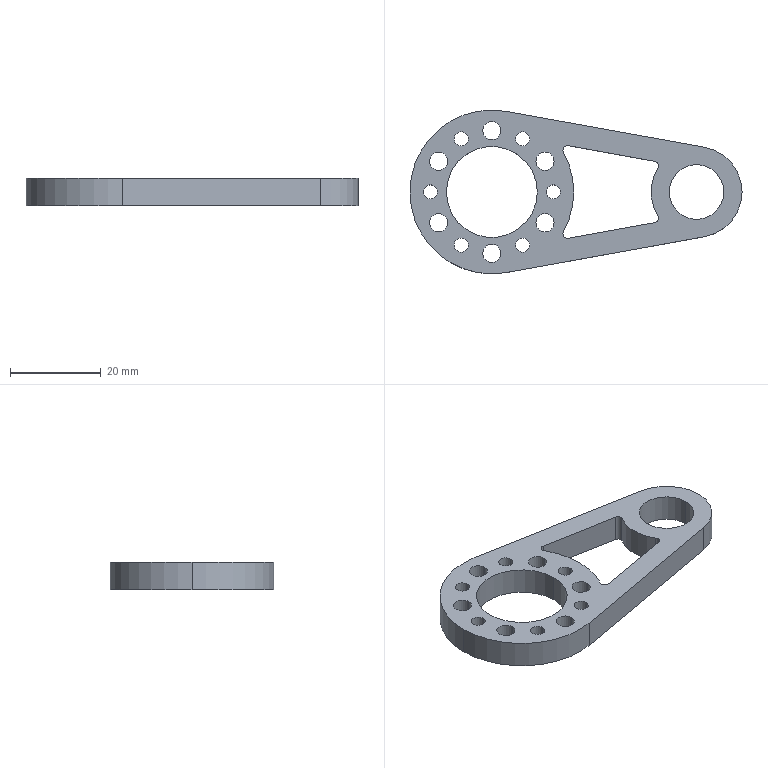Part | SolidWorks | features Extrusion 1, Fillet 1, ICE 1 | 1 solid | 46 faces | box 73 x 36 x 6 mm | volume 6499 mm3 | cylinder 40 | plane 6 | commonest cylinder face diameters 3.1 x12 4 x12 2 x6 20 x4 36 x4 12 x2
STEP:
#1=CARTESIAN_POINT('',(36.627,5.758,0.));
#2=VERTEX_POINT('',#1);
#3=CARTESIAN_POINT('',(35.805,6.742,0.));
#4=VERTEX_POINT('',#3);
#5=CARTESIAN_POINT('',(35.627,5.758,0.));
#6=DIRECTION('',(0.,0.,1.));
#7=DIRECTION('',(1.,0.,0.));
#8=AXIS2_PLACEMENT_3D('',#5,#6,#7);
#9=CIRCLE('',#8,1.);
#10=EDGE_CURVE('',#2,#4,#9,.T.);
#11=ORIENTED_EDGE('',*,*,#10,.F.);
#12=CARTESIAN_POINT('',(36.627,5.758,6.));
#13=VERTEX_POINT('',#12);
#14=CARTESIAN_POINT('',(36.627,5.758,0.));
#15=DIRECTION('',(0.,0.,1.));
#16=VECTOR('',#15,1000.);
#17=LINE('',#14,#16);
#18=EDGE_CURVE('',#2,#13,#17,.T.);
#19=ORIENTED_EDGE('',*,*,#18,.T.);
#20=CARTESIAN_POINT('',(35.805,6.742,6.));
#21=VERTEX_POINT('',#20);
#22=CARTESIAN_POINT('',(35.627,5.758,6.));
#23=DIRECTION('',(0.,0.,-1.));
#24=DIRECTION('',(1.,0.,0.));
#25=AXIS2_PLACEMENT_3D('',#22,#23,#24);
#26=CIRCLE('',#25,1.);
#27=EDGE_CURVE('',#21,#13,#26,.T.);
#28=ORIENTED_EDGE('',*,*,#27,.F.);
#29=CARTESIAN_POINT('',(35.805,6.742,6.));
#30=DIRECTION('',(0.,0.,1.));
#31=VECTOR('',#30,1000.);
#32=LINE('',#29,#31);
#33=EDGE_CURVE('',#4,#21,#32,.T.);
#34=ORIENTED_EDGE('',*,*,#33,.F.);
#35=EDGE_LOOP('',(#11,#19,#28,#34));
#36=FACE_OUTER_BOUND('',#35,.T.);
#37=CARTESIAN_POINT('',(35.627,5.758,0.));
#38=DIRECTION('',(0.,0.,1.));
#39=DIRECTION('',(1.,0.,0.));
#40=AXIS2_PLACEMENT_3D('',#37,#38,#39);
#41=CYLINDRICAL_SURFACE('',#40,1.);
#42=ADVANCED_FACE('',(#36),#41,.F.);
#43=CARTESIAN_POINT('',(36.627,-5.758,0.));
#44=VERTEX_POINT('',#43);
#45=CARTESIAN_POINT('',(36.479,-5.235,0.));
#46=VERTEX_POINT('',#45);
#47=CARTESIAN_POINT('',(35.627,-5.758,0.));
#48=DIRECTION('',(0.,0.,1.));
#49=DIRECTION('',(1.,0.,0.));
#50=AXIS2_PLACEMENT_3D('',#47,#48,#49);
#51=CIRCLE('',#50,1.);
#52=EDGE_CURVE('',#44,#46,#51,.T.);
#53=ORIENTED_EDGE('',*,*,#52,.F.);
#54=CARTESIAN_POINT('',(36.627,-5.758,6.));
#55=VERTEX_POINT('',#54);
#56=CARTESIAN_POINT('',(36.627,-5.758,0.));
#57=DIRECTION('',(0.,0.,1.));
#58=VECTOR('',#57,1000.);
#59=LINE('',#56,#58);
#60=EDGE_CURVE('',#44,#55,#59,.T.);
#61=ORIENTED_EDGE('',*,*,#60,.T.);
#62=CARTESIAN_POINT('',(36.479,-5.235,6.));
#63=VERTEX_POINT('',#62);
#64=CARTESIAN_POINT('',(35.627,-5.758,6.));
#65=DIRECTION('',(0.,0.,-1.));
#66=DIRECTION('',(1.,0.,0.));
#67=AXIS2_PLACEMENT_3D('',#64,#65,#66);
#68=CIRCLE('',#67,1.);
#69=EDGE_CURVE('',#63,#55,#68,.T.);
#70=ORIENTED_EDGE('',*,*,#69,.F.);
#71=CARTESIAN_POINT('',(36.479,-5.235,0.));
#72=DIRECTION('',(0.,0.,1.));
#73=VECTOR('',#72,1000.);
#74=LINE('',#71,#73);
#75=EDGE_CURVE('',#46,#63,#74,.T.);
#76=ORIENTED_EDGE('',*,*,#75,.F.);
#77=EDGE_LOOP('',(#53,#61,#70,#76));
#78=FACE_OUTER_BOUND('',#77,.T.);
#79=CARTESIAN_POINT('',(35.627,-5.758,0.));
#80=DIRECTION('',(0.,0.,1.));
#81=DIRECTION('',(1.,0.,0.));
#82=AXIS2_PLACEMENT_3D('',#79,#80,#81);
#83=CYLINDRICAL_SURFACE('',#82,1.);
#84=ADVANCED_FACE('',(#78),#83,.F.);
#85=CARTESIAN_POINT('',(15.754,-8.706,0.));
#86=VERTEX_POINT('',#85);
#87=CARTESIAN_POINT('',(18.,0.,0.));
#88=VERTEX_POINT('',#87);
#89=CARTESIAN_POINT('',(0.,0.,0.));
#90=DIRECTION('',(0.,0.,1.));
#91=DIRECTION('',(1.,0.,0.));
#92=AXIS2_PLACEMENT_3D('',#89,#90,#91);
#93=CIRCLE('',#92,18.);
#94=EDGE_CURVE('',#86,#88,#93,.T.);
#95=ORIENTED_EDGE('',*,*,#94,.T.);
#96=CARTESIAN_POINT('',(18.,0.,6.));
#97=VERTEX_POINT('',#96);
#98=CARTESIAN_POINT('',(18.,0.,0.));
#99=DIRECTION('',(0.,0.,1.));
#100=VECTOR('',#99,1000.);
#101=LINE('',#98,#100);
#102=EDGE_CURVE('',#88,#97,#101,.T.);
#103=ORIENTED_EDGE('',*,*,#102,.T.);
#104=CARTESIAN_POINT('',(15.754,-8.706,6.));
#105=VERTEX_POINT('',#104);
#106=CARTESIAN_POINT('',(0.,0.,6.));
#107=DIRECTION('',(0.,0.,1.));
#108=DIRECTION('',(1.,0.,0.));
#109=AXIS2_PLACEMENT_3D('',#106,#107,#108);
#110=CIRCLE('',#109,18.);
#111=EDGE_CURVE('',#105,#97,#110,.T.);
#112=ORIENTED_EDGE('',*,*,#111,.F.);
#113=CARTESIAN_POINT('',(15.754,-8.706,0.));
#114=DIRECTION('',(0.,0.,-1.));
#115=VECTOR('',#114,1000.);
#116=LINE('',#113,#115);
#117=EDGE_CURVE('',#105,#86,#116,.T.);
#118=ORIENTED_EDGE('',*,*,#117,.T.);
#119=EDGE_LOOP('',(#95,#103,#112,#118));
#120=FACE_OUTER_BOUND('',#119,.T.);
#121=CARTESIAN_POINT('',(0.,0.,0.));
#122=DIRECTION('',(0.,0.,1.));
#123=DIRECTION('',(1.,0.,0.));
#124=AXIS2_PLACEMENT_3D('',#121,#122,#123);
#125=CYLINDRICAL_SURFACE('',#124,18.);
#126=ADVANCED_FACE('',(#120),#125,.T.);
#127=CARTESIAN_POINT('',(39.,0.,6.));
#128=VERTEX_POINT('',#127);
#129=CARTESIAN_POINT('',(51.,0.,6.));
#130=VERTEX_POINT('',#129);
#131=CARTESIAN_POINT('',(45.,0.,6.));
#132=DIRECTION('',(0.,0.,1.));
#133=DIRECTION('',(1.,0.,0.));
#134=AXIS2_PLACEMENT_3D('',#131,#132,#133);
#135=CIRCLE('',#134,6.);
#136=EDGE_CURVE('',#128,#130,#135,.T.);
#137=ORIENTED_EDGE('',*,*,#136,.T.);
#138=CARTESIAN_POINT('',(51.,0.,0.));
#139=VERTEX_POINT('',#138);
#140=CARTESIAN_POINT('',(51.,0.,6.));
#141=DIRECTION('',(0.,0.,-1.));
#142=VECTOR('',#141,1000.);
#143=LINE('',#140,#142);
#144=EDGE_CURVE('',#130,#139,#143,.T.);
#145=ORIENTED_EDGE('',*,*,#144,.T.);
#146=CARTESIAN_POINT('',(39.,0.,0.));
#147=VERTEX_POINT('',#146);
#148=CARTESIAN_POINT('',(45.,0.,0.));
#149=DIRECTION('',(0.,0.,1.));
#150=DIRECTION('',(1.,0.,0.));
#151=AXIS2_PLACEMENT_3D('',#148,#149,#150);
#152=CIRCLE('',#151,6.);
#153=EDGE_CURVE('',#147,#139,#152,.T.);
#154=ORIENTED_EDGE('',*,*,#153,.F.);
#155=CARTESIAN_POINT('',(39.,0.,6.));
#156=DIRECTION('',(0.,0.,-1.));
#157=VECTOR('',#156,1000.);
#158=LINE('',#155,#157);
#159=EDGE_CURVE('',#128,#147,#158,.T.);
#160=ORIENTED_EDGE('',*,*,#159,.F.);
#161=EDGE_LOOP('',(#137,#145,#154,#160));
#162=FACE_OUTER_BOUND('',#161,.T.);
#163=CARTESIAN_POINT('',(45.,0.,6.));
#164=DIRECTION('',(0.,0.,-1.));
#165=DIRECTION('',(-1.,0.,0.));
#166=AXIS2_PLACEMENT_3D('',#163,#164,#165);
#167=CYLINDRICAL_SURFACE('',#166,6.);
#168=ADVANCED_FACE('',(#162),#167,.F.);
#169=CARTESIAN_POINT('',(-13.691,6.75,6.));
#170=VERTEX_POINT('',#169);
#171=CARTESIAN_POINT('',(-9.691,6.75,6.));
#172=VERTEX_POINT('',#171);
#173=CARTESIAN_POINT('',(-11.691,6.75,6.));
#174=DIRECTION('',(0.,0.,1.));
#175=DIRECTION('',(1.,0.,0.));
#176=AXIS2_PLACEMENT_3D('',#173,#174,#175);
#177=CIRCLE('',#176,2.);
#178=EDGE_CURVE('',#170,#172,#177,.T.);
#179=ORIENTED_EDGE('',*,*,#178,.T.);
#180=CARTESIAN_POINT('',(-9.691,6.75,0.));
#181=VERTEX_POINT('',#180);
#182=CARTESIAN_POINT('',(-9.691,6.75,6.));
#183=DIRECTION('',(0.,0.,-1.));
#184=VECTOR('',#183,1000.);
#185=LINE('',#182,#184);
#186=EDGE_CURVE('',#172,#181,#185,.T.);
#187=ORIENTED_EDGE('',*,*,#186,.T.);
#188=CARTESIAN_POINT('',(-13.691,6.75,0.));
#189=VERTEX_POINT('',#188);
#190=CARTESIAN_POINT('',(-11.691,6.75,0.));
#191=DIRECTION('',(0.,0.,1.));
#192=DIRECTION('',(1.,0.,0.));
#193=AXIS2_PLACEMENT_3D('',#190,#191,#192);
#194=CIRCLE('',#193,2.);
#195=EDGE_CURVE('',#189,#181,#194,.T.);
#196=ORIENTED_EDGE('',*,*,#195,.F.);
#197=CARTESIAN_POINT('',(-13.691,6.75,6.));
#198=DIRECTION('',(0.,0.,-1.));
#199=VECTOR('',#198,1000.);
#200=LINE('',#197,#199);
#201=EDGE_CURVE('',#170,#189,#200,.T.);
#202=ORIENTED_EDGE('',*,*,#201,.F.);
#203=EDGE_LOOP('',(#179,#187,#196,#202));
#204=FACE_OUTER_BOUND('',#203,.T.);
#205=CARTESIAN_POINT('',(-11.691,6.75,6.));
#206=DIRECTION('',(0.,0.,-1.));
#207=DIRECTION('',(-1.,0.,0.));
#208=AXIS2_PLACEMENT_3D('',#205,#206,#207);
#209=CYLINDRICAL_SURFACE('',#208,2.);
#210=ADVANCED_FACE('',(#204),#209,.F.);
#211=CARTESIAN_POINT('',(-13.691,-6.75,6.));
#212=VERTEX_POINT('',#211);
#213=CARTESIAN_POINT('',(-9.691,-6.75,6.));
#214=VERTEX_POINT('',#213);
#215=CARTESIAN_POINT('',(-11.691,-6.75,6.));
#216=DIRECTION('',(0.,0.,1.));
#217=DIRECTION('',(1.,0.,0.));
#218=AXIS2_PLACEMENT_3D('',#215,#216,#217);
#219=CIRCLE('',#218,2.);
#220=EDGE_CURVE('',#212,#214,#219,.T.);
#221=ORIENTED_EDGE('',*,*,#220,.T.);
#222=CARTESIAN_POINT('',(-9.691,-6.75,0.));
#223=VERTEX_POINT('',#222);
#224=CARTESIAN_POINT('',(-9.691,-6.75,6.));
#225=DIRECTION('',(0.,0.,-1.));
#226=VECTOR('',#225,1000.);
#227=LINE('',#224,#226);
#228=EDGE_CURVE('',#214,#223,#227,.T.);
#229=ORIENTED_EDGE('',*,*,#228,.T.);
#230=CARTESIAN_POINT('',(-13.691,-6.75,0.));
#231=VERTEX_POINT('',#230);
#232=CARTESIAN_POINT('',(-11.691,-6.75,0.));
#233=DIRECTION('',(0.,0.,1.));
#234=DIRECTION('',(1.,0.,0.));
#235=AXIS2_PLACEMENT_3D('',#232,#233,#234);
#236=CIRCLE('',#235,2.);
#237=EDGE_CURVE('',#231,#223,#236,.T.);
#238=ORIENTED_EDGE('',*,*,#237,.F.);
#239=CARTESIAN_POINT('',(-13.691,-6.75,6.));
#240=DIRECTION('',(0.,0.,-1.));
#241=VECTOR('',#240,1000.);
#242=LINE('',#239,#241);
#243=EDGE_CURVE('',#212,#231,#242,.T.);
#244=ORIENTED_EDGE('',*,*,#243,.F.);
#245=EDGE_LOOP('',(#221,#229,#238,#244));
#246=FACE_OUTER_BOUND('',#245,.T.);
#247=CARTESIAN_POINT('',(-11.691,-6.75,6.));
#248=DIRECTION('',(0.,0.,-1.));
#249=DIRECTION('',(-1.,0.,0.));
#250=AXIS2_PLACEMENT_3D('',#247,#248,#249);
#251=CYLINDRICAL_SURFACE('',#250,2.);
#252=ADVANCED_FACE('',(#246),#251,.F.);
#253=CARTESIAN_POINT('',(-2.,-13.5,6.));
#254=VERTEX_POINT('',#253);
#255=CARTESIAN_POINT('',(2.,-13.5,6.));
#256=VERTEX_POINT('',#255);
#257=CARTESIAN_POINT('',(0.,-13.5,6.));
#258=DIRECTION('',(0.,0.,1.));
#259=DIRECTION('',(1.,0.,0.));
#260=AXIS2_PLACEMENT_3D('',#257,#258,#259);
#261=CIRCLE('',#260,2.);
#262=EDGE_CURVE('',#254,#256,#261,.T.);
#263=ORIENTED_EDGE('',*,*,#262,.T.);
#264=CARTESIAN_POINT('',(2.,-13.5,0.));
#265=VERTEX_POINT('',#264);
#266=CARTESIAN_POINT('',(2.,-13.5,6.));
#267=DIRECTION('',(0.,0.,-1.));
#268=VECTOR('',#267,1000.);
#269=LINE('',#266,#268);
#270=EDGE_CURVE('',#256,#265,#269,.T.);
#271=ORIENTED_EDGE('',*,*,#270,.T.);
#272=CARTESIAN_POINT('',(-2.,-13.5,0.));
#273=VERTEX_POINT('',#272);
#274=CARTESIAN_POINT('',(0.,-13.5,0.));
#275=DIRECTION('',(0.,0.,1.));
#276=DIRECTION('',(1.,0.,0.));
#277=AXIS2_PLACEMENT_3D('',#274,#275,#276);
#278=CIRCLE('',#277,2.);
#279=EDGE_CURVE('',#273,#265,#278,.T.);
#280=ORIENTED_EDGE('',*,*,#279,.F.);
#281=CARTESIAN_POINT('',(-2.,-13.5,6.));
#282=DIRECTION('',(0.,0.,-1.));
#283=VECTOR('',#282,1000.);
#284=LINE('',#281,#283);
#285=EDGE_CURVE('',#254,#273,#284,.T.);
#286=ORIENTED_EDGE('',*,*,#285,.F.);
#287=EDGE_LOOP('',(#263,#271,#280,#286));
#288=FACE_OUTER_BOUND('',#287,.T.);
#289=CARTESIAN_POINT('',(0.,-13.5,6.));
#290=DIRECTION('',(0.,0.,-1.));
#291=DIRECTION('',(-1.,0.,0.));
#292=AXIS2_PLACEMENT_3D('',#289,#290,#291);
#293=CYLINDRICAL_SURFACE('',#292,2.);
#294=ADVANCED_FACE('',(#288),#293,.F.);
#295=CARTESIAN_POINT('',(9.691,-6.75,6.));
#296=VERTEX_POINT('',#295);
#297=CARTESIAN_POINT('',(13.691,-6.75,6.));
#298=VERTEX_POINT('',#297);
#299=CARTESIAN_POINT('',(11.691,-6.75,6.));
#300=DIRECTION('',(0.,0.,1.));
#301=DIRECTION('',(1.,0.,0.));
#302=AXIS2_PLACEMENT_3D('',#299,#300,#301);
#303=CIRCLE('',#302,2.);
#304=EDGE_CURVE('',#296,#298,#303,.T.);
#305=ORIENTED_EDGE('',*,*,#304,.T.);
#306=CARTESIAN_POINT('',(13.691,-6.75,0.));
#307=VERTEX_POINT('',#306);
#308=CARTESIAN_POINT('',(13.691,-6.75,6.));
#309=DIRECTION('',(0.,0.,-1.));
#310=VECTOR('',#309,1000.);
#311=LINE('',#308,#310);
#312=EDGE_CURVE('',#298,#307,#311,.T.);
#313=ORIENTED_EDGE('',*,*,#312,.T.);
#314=CARTESIAN_POINT('',(9.691,-6.75,0.));
#315=VERTEX_POINT('',#314);
#316=CARTESIAN_POINT('',(11.691,-6.75,0.));
#317=DIRECTION('',(0.,0.,1.));
#318=DIRECTION('',(1.,0.,0.));
#319=AXIS2_PLACEMENT_3D('',#316,#317,#318);
#320=CIRCLE('',#319,2.);
#321=EDGE_CURVE('',#315,#307,#320,.T.);
#322=ORIENTED_EDGE('',*,*,#321,.F.);
#323=CARTESIAN_POINT('',(9.691,-6.75,6.));
#324=DIRECTION('',(0.,0.,-1.));
#325=VECTOR('',#324,1000.);
#326=LINE('',#323,#325);
#327=EDGE_CURVE('',#296,#315,#326,.T.);
#328=ORIENTED_EDGE('',*,*,#327,.F.);
#329=EDGE_LOOP('',(#305,#313,#322,#328));
#330=FACE_OUTER_BOUND('',#329,.T.);
#331=CARTESIAN_POINT('',(11.691,-6.75,6.));
#332=DIRECTION('',(0.,0.,-1.));
#333=DIRECTION('',(-1.,0.,0.));
#334=AXIS2_PLACEMENT_3D('',#331,#332,#333);
#335=CYLINDRICAL_SURFACE('',#334,2.);
#336=ADVANCED_FACE('',(#330),#335,.F.);
#337=CARTESIAN_POINT('',(9.691,6.75,6.));
#338=VERTEX_POINT('',#337);
#339=CARTESIAN_POINT('',(13.691,6.75,6.));
#340=VERTEX_POINT('',#339);
#341=CARTESIAN_POINT('',(11.691,6.75,6.));
#342=DIRECTION('',(0.,0.,1.));
#343=DIRECTION('',(1.,0.,0.));
#344=AXIS2_PLACEMENT_3D('',#341,#342,#343);
#345=CIRCLE('',#344,2.);
#346=EDGE_CURVE('',#338,#340,#345,.T.);
#347=ORIENTED_EDGE('',*,*,#346,.T.);
#348=CARTESIAN_POINT('',(13.691,6.75,0.));
#349=VERTEX_POINT('',#348);
#350=CARTESIAN_POINT('',(13.691,6.75,6.));
#351=DIRECTION('',(0.,0.,-1.));
#352=VECTOR('',#351,1000.);
#353=LINE('',#350,#352);
#354=EDGE_CURVE('',#340,#349,#353,.T.);
#355=ORIENTED_EDGE('',*,*,#354,.T.);
#356=CARTESIAN_POINT('',(9.691,6.75,0.));
#357=VERTEX_POINT('',#356);
#358=CARTESIAN_POINT('',(11.691,6.75,0.));
#359=DIRECTION('',(0.,0.,1.));
#360=DIRECTION('',(1.,0.,0.));
#361=AXIS2_PLACEMENT_3D('',#358,#359,#360);
#362=CIRCLE('',#361,2.);
#363=EDGE_CURVE('',#357,#349,#362,.T.);
#364=ORIENTED_EDGE('',*,*,#363,.F.);
#365=CARTESIAN_POINT('',(9.691,6.75,6.));
#366=DIRECTION('',(0.,0.,-1.));
#367=VECTOR('',#366,1000.);
#368=LINE('',#365,#367);
#369=EDGE_CURVE('',#338,#357,#368,.T.);
#370=ORIENTED_EDGE('',*,*,#369,.F.);
#371=EDGE_LOOP('',(#347,#355,#364,#370));
#372=FACE_OUTER_BOUND('',#371,.T.);
#373=CARTESIAN_POINT('',(11.691,6.75,6.));
#374=DIRECTION('',(0.,0.,-1.));
#375=DIRECTION('',(-1.,0.,0.));
#376=AXIS2_PLACEMENT_3D('',#373,#374,#375);
#377=CYLINDRICAL_SURFACE('',#376,2.);
#378=ADVANCED_FACE('',(#372),#377,.F.);
#379=CARTESIAN_POINT('',(-2.,13.5,6.));
#380=VERTEX_POINT('',#379);
#381=CARTESIAN_POINT('',(2.,13.5,6.));
#382=VERTEX_POINT('',#381);
#383=CARTESIAN_POINT('',(0.,13.5,6.));
#384=DIRECTION('',(0.,0.,1.));
#385=DIRECTION('',(1.,0.,0.));
#386=AXIS2_PLACEMENT_3D('',#383,#384,#385);
#387=CIRCLE('',#386,2.);
#388=EDGE_CURVE('',#380,#382,#387,.T.);
#389=ORIENTED_EDGE('',*,*,#388,.T.);
#390=CARTESIAN_POINT('',(2.,13.5,0.));
#391=VERTEX_POINT('',#390);
#392=CARTESIAN_POINT('',(2.,13.5,6.));
#393=DIRECTION('',(0.,0.,-1.));
#394=VECTOR('',#393,1000.);
#395=LINE('',#392,#394);
#396=EDGE_CURVE('',#382,#391,#395,.T.);
#397=ORIENTED_EDGE('',*,*,#396,.T.);
#398=CARTESIAN_POINT('',(-2.,13.5,0.));
#399=VERTEX_POINT('',#398);
#400=CARTESIAN_POINT('',(0.,13.5,0.));
#401=DIRECTION('',(0.,0.,1.));
#402=DIRECTION('',(1.,0.,0.));
#403=AXIS2_PLACEMENT_3D('',#400,#401,#402);
#404=CIRCLE('',#403,2.);
#405=EDGE_CURVE('',#399,#391,#404,.T.);
#406=ORIENTED_EDGE('',*,*,#405,.F.);
#407=CARTESIAN_POINT('',(-2.,13.5,6.));
#408=DIRECTION('',(0.,0.,-1.));
#409=VECTOR('',#408,1000.);
#410=LINE('',#407,#409);
#411=EDGE_CURVE('',#380,#399,#410,.T.);
#412=ORIENTED_EDGE('',*,*,#411,.F.);
#413=EDGE_LOOP('',(#389,#397,#406,#412));
#414=FACE_OUTER_BOUND('',#413,.T.);
#415=CARTESIAN_POINT('',(0.,13.5,6.));
#416=DIRECTION('',(0.,0.,-1.));
#417=DIRECTION('',(-1.,0.,0.));
#418=AXIS2_PLACEMENT_3D('',#415,#416,#417);
#419=CYLINDRICAL_SURFACE('',#418,2.);
#420=ADVANCED_FACE('',(#414),#419,.F.);
#421=CARTESIAN_POINT('',(-10.,0.,6.));
#422=VERTEX_POINT('',#421);
#423=CARTESIAN_POINT('',(10.,0.,6.));
#424=VERTEX_POINT('',#423);
#425=CARTESIAN_POINT('',(0.,0.,6.));
#426=DIRECTION('',(0.,0.,1.));
#427=DIRECTION('',(1.,0.,0.));
#428=AXIS2_PLACEMENT_3D('',#425,#426,#427);
#429=CIRCLE('',#428,10.);
#430=EDGE_CURVE('',#422,#424,#429,.T.);
#431=ORIENTED_EDGE('',*,*,#430,.T.);
#432=CARTESIAN_POINT('',(10.,0.,0.));
#433=VERTEX_POINT('',#432);
#434=CARTESIAN_POINT('',(10.,0.,6.));
#435=DIRECTION('',(0.,0.,-1.));
#436=VECTOR('',#435,1000.);
#437=LINE('',#434,#436);
#438=EDGE_CURVE('',#424,#433,#437,.T.);
#439=ORIENTED_EDGE('',*,*,#438,.T.);
#440=CARTESIAN_POINT('',(-10.,0.,0.));
#441=VERTEX_POINT('',#440);
#442=CARTESIAN_POINT('',(0.,0.,0.));
#443=DIRECTION('',(0.,0.,1.));
#444=DIRECTION('',(1.,0.,0.));
#445=AXIS2_PLACEMENT_3D('',#442,#443,#444);
#446=CIRCLE('',#445,10.);
#447=EDGE_CURVE('',#441,#433,#446,.T.);
#448=ORIENTED_EDGE('',*,*,#447,.F.);
#449=CARTESIAN_POINT('',(-10.,0.,6.));
#450=DIRECTION('',(0.,0.,-1.));
#451=VECTOR('',#450,1000.);
#452=LINE('',#449,#451);
#453=EDGE_CURVE('',#422,#441,#452,.T.);
#454=ORIENTED_EDGE('',*,*,#453,.F.);
#455=EDGE_LOOP('',(#431,#439,#448,#454));
#456=FACE_OUTER_BOUND('',#455,.T.);
#457=CARTESIAN_POINT('',(0.,0.,6.));
#458=DIRECTION('',(0.,0.,-1.));
#459=DIRECTION('',(-1.,0.,0.));
#460=AXIS2_PLACEMENT_3D('',#457,#458,#459);
#461=CYLINDRICAL_SURFACE('',#460,10.);
#462=ADVANCED_FACE('',(#456),#461,.F.);
#463=CARTESIAN_POINT('',(11.95,0.,6.));
#464=VERTEX_POINT('',#463);
#465=CARTESIAN_POINT('',(15.05,0.,6.));
#466=VERTEX_POINT('',#465);
#467=CARTESIAN_POINT('',(13.5,0.,6.));
#468=DIRECTION('',(0.,0.,1.));
#469=DIRECTION('',(1.,0.,0.));
#470=AXIS2_PLACEMENT_3D('',#467,#468,#469);
#471=CIRCLE('',#470,1.55);
#472=EDGE_CURVE('',#464,#466,#471,.T.);
#473=ORIENTED_EDGE('',*,*,#472,.T.);
#474=CARTESIAN_POINT('',(15.05,0.,0.));
#475=VERTEX_POINT('',#474);
#476=CARTESIAN_POINT('',(15.05,0.,6.));
#477=DIRECTION('',(0.,0.,-1.));
#478=VECTOR('',#477,1000.);
#479=LINE('',#476,#478);
#480=EDGE_CURVE('',#466,#475,#479,.T.);
#481=ORIENTED_EDGE('',*,*,#480,.T.);
#482=CARTESIAN_POINT('',(11.95,0.,0.));
#483=VERTEX_POINT('',#482);
#484=CARTESIAN_POINT('',(13.5,0.,0.));
#485=DIRECTION('',(0.,0.,1.));
#486=DIRECTION('',(1.,0.,0.));
#487=AXIS2_PLACEMENT_3D('',#484,#485,#486);
#488=CIRCLE('',#487,1.55);
#489=EDGE_CURVE('',#483,#475,#488,.T.);
#490=ORIENTED_EDGE('',*,*,#489,.F.);
#491=CARTESIAN_POINT('',(11.95,0.,6.));
#492=DIRECTION('',(0.,0.,-1.));
#493=VECTOR('',#492,1000.);
#494=LINE('',#491,#493);
#495=EDGE_CURVE('',#464,#483,#494,.T.);
#496=ORIENTED_EDGE('',*,*,#495,.F.);
#497=EDGE_LOOP('',(#473,#481,#490,#496));
#498=FACE_OUTER_BOUND('',#497,.T.);
#499=CARTESIAN_POINT('',(13.5,0.,6.));
#500=DIRECTION('',(0.,0.,-1.));
#501=DIRECTION('',(-1.,0.,0.));
#502=AXIS2_PLACEMENT_3D('',#499,#500,#501);
#503=CYLINDRICAL_SURFACE('',#502,1.55);
#504=ADVANCED_FACE('',(#498),#503,.F.);
#505=CARTESIAN_POINT('',(5.2,-11.691,6.));
#506=VERTEX_POINT('',#505);
#507=CARTESIAN_POINT('',(8.3,-11.691,6.));
#508=VERTEX_POINT('',#507);
#509=CARTESIAN_POINT('',(6.75,-11.691,6.));
#510=DIRECTION('',(0.,0.,1.));
#511=DIRECTION('',(1.,0.,0.));
#512=AXIS2_PLACEMENT_3D('',#509,#510,#511);
#513=CIRCLE('',#512,1.55);
#514=EDGE_CURVE('',#506,#508,#513,.T.);
#515=ORIENTED_EDGE('',*,*,#514,.T.);
#516=CARTESIAN_POINT('',(8.3,-11.691,0.));
#517=VERTEX_POINT('',#516);
#518=CARTESIAN_POINT('',(8.3,-11.691,6.));
#519=DIRECTION('',(0.,0.,-1.));
#520=VECTOR('',#519,1000.);
#521=LINE('',#518,#520);
#522=EDGE_CURVE('',#508,#517,#521,.T.);
#523=ORIENTED_EDGE('',*,*,#522,.T.);
#524=CARTESIAN_POINT('',(5.2,-11.691,0.));
#525=VERTEX_POINT('',#524);
#526=CARTESIAN_POINT('',(6.75,-11.691,0.));
#527=DIRECTION('',(0.,0.,1.));
#528=DIRECTION('',(1.,0.,0.));
#529=AXIS2_PLACEMENT_3D('',#526,#527,#528);
#530=CIRCLE('',#529,1.55);
#531=EDGE_CURVE('',#525,#517,#530,.T.);
#532=ORIENTED_EDGE('',*,*,#531,.F.);
#533=CARTESIAN_POINT('',(5.2,-11.691,6.));
#534=DIRECTION('',(0.,0.,-1.));
#535=VECTOR('',#534,1000.);
#536=LINE('',#533,#535);
#537=EDGE_CURVE('',#506,#525,#536,.T.);
#538=ORIENTED_EDGE('',*,*,#537,.F.);
#539=EDGE_LOOP('',(#515,#523,#532,#538));
#540=FACE_OUTER_BOUND('',#539,.T.);
#541=CARTESIAN_POINT('',(6.75,-11.691,6.));
#542=DIRECTION('',(0.,0.,-1.));
#543=DIRECTION('',(-1.,0.,0.));
#544=AXIS2_PLACEMENT_3D('',#541,#542,#543);
#545=CYLINDRICAL_SURFACE('',#544,1.55);
#546=ADVANCED_FACE('',(#540),#545,.F.);
#547=CARTESIAN_POINT('',(-8.3,-11.691,6.));
#548=VERTEX_POINT('',#547);
#549=CARTESIAN_POINT('',(-5.2,-11.691,6.));
#550=VERTEX_POINT('',#549);
#551=CARTESIAN_POINT('',(-6.75,-11.691,6.));
#552=DIRECTION('',(0.,0.,1.));
#553=DIRECTION('',(1.,0.,0.));
#554=AXIS2_PLACEMENT_3D('',#551,#552,#553);
#555=CIRCLE('',#554,1.55);
#556=EDGE_CURVE('',#548,#550,#555,.T.);
#557=ORIENTED_EDGE('',*,*,#556,.T.);
#558=CARTESIAN_POINT('',(-5.2,-11.691,0.));
#559=VERTEX_POINT('',#558);
#560=CARTESIAN_POINT('',(-5.2,-11.691,6.));
#561=DIRECTION('',(0.,0.,-1.));
#562=VECTOR('',#561,1000.);
#563=LINE('',#560,#562);
#564=EDGE_CURVE('',#550,#559,#563,.T.);
#565=ORIENTED_EDGE('',*,*,#564,.T.);
#566=CARTESIAN_POINT('',(-8.3,-11.691,0.));
#567=VERTEX_POINT('',#566);
#568=CARTESIAN_POINT('',(-6.75,-11.691,0.));
#569=DIRECTION('',(0.,0.,1.));
#570=DIRECTION('',(1.,0.,0.));
#571=AXIS2_PLACEMENT_3D('',#568,#569,#570);
#572=CIRCLE('',#571,1.55);
#573=EDGE_CURVE('',#567,#559,#572,.T.);
#574=ORIENTED_EDGE('',*,*,#573,.F.);
#575=CARTESIAN_POINT('',(-8.3,-11.691,6.));
#576=DIRECTION('',(0.,0.,-1.));
#577=VECTOR('',#576,1000.);
#578=LINE('',#575,#577);
#579=EDGE_CURVE('',#548,#567,#578,.T.);
#580=ORIENTED_EDGE('',*,*,#579,.F.);
#581=EDGE_LOOP('',(#557,#565,#574,#580));
#582=FACE_OUTER_BOUND('',#581,.T.);
#583=CARTESIAN_POINT('',(-6.75,-11.691,6.));
#584=DIRECTION('',(0.,0.,-1.));
#585=DIRECTION('',(-1.,0.,0.));
#586=AXIS2_PLACEMENT_3D('',#583,#584,#585);
#587=CYLINDRICAL_SURFACE('',#586,1.55);
#588=ADVANCED_FACE('',(#582),#587,.F.);
#589=CARTESIAN_POINT('',(-15.05,0.,6.));
#590=VERTEX_POINT('',#589);
#591=CARTESIAN_POINT('',(-11.95,0.,6.));
#592=VERTEX_POINT('',#591);
#593=CARTESIAN_POINT('',(-13.5,0.,6.));
#594=DIRECTION('',(0.,0.,1.));
#595=DIRECTION('',(1.,0.,0.));
#596=AXIS2_PLACEMENT_3D('',#593,#594,#595);
#597=CIRCLE('',#596,1.55);
#598=EDGE_CURVE('',#590,#592,#597,.T.);
#599=ORIENTED_EDGE('',*,*,#598,.T.);
#600=CARTESIAN_POINT('',(-11.95,0.,0.));
#601=VERTEX_POINT('',#600);
#602=CARTESIAN_POINT('',(-11.95,0.,6.));
#603=DIRECTION('',(0.,0.,-1.));
#604=VECTOR('',#603,1000.);
#605=LINE('',#602,#604);
#606=EDGE_CURVE('',#592,#601,#605,.T.);
#607=ORIENTED_EDGE('',*,*,#606,.T.);
#608=CARTESIAN_POINT('',(-15.05,0.,0.));
#609=VERTEX_POINT('',#608);
#610=CARTESIAN_POINT('',(-13.5,0.,0.));
#611=DIRECTION('',(0.,0.,1.));
#612=DIRECTION('',(1.,0.,0.));
#613=AXIS2_PLACEMENT_3D('',#610,#611,#612);
#614=CIRCLE('',#613,1.55);
#615=EDGE_CURVE('',#609,#601,#614,.T.);
#616=ORIENTED_EDGE('',*,*,#615,.F.);
#617=CARTESIAN_POINT('',(-15.05,0.,6.));
#618=DIRECTION('',(0.,0.,-1.));
#619=VECTOR('',#618,1000.);
#620=LINE('',#617,#619);
#621=EDGE_CURVE('',#590,#609,#620,.T.);
#622=ORIENTED_EDGE('',*,*,#621,.F.);
#623=EDGE_LOOP('',(#599,#607,#616,#622));
#624=FACE_OUTER_BOUND('',#623,.T.);
#625=CARTESIAN_POINT('',(-13.5,0.,6.));
#626=DIRECTION('',(0.,0.,-1.));
#627=DIRECTION('',(-1.,0.,0.));
#628=AXIS2_PLACEMENT_3D('',#625,#626,#627);
#629=CYLINDRICAL_SURFACE('',#628,1.55);
#630=ADVANCED_FACE('',(#624),#629,.F.);
#631=CARTESIAN_POINT('',(-8.3,11.691,6.));
#632=VERTEX_POINT('',#631);
#633=CARTESIAN_POINT('',(-5.2,11.691,6.));
#634=VERTEX_POINT('',#633);
#635=CARTESIAN_POINT('',(-6.75,11.691,6.));
#636=DIRECTION('',(0.,0.,1.));
#637=DIRECTION('',(1.,0.,0.));
#638=AXIS2_PLACEMENT_3D('',#635,#636,#637);
#639=CIRCLE('',#638,1.55);
#640=EDGE_CURVE('',#632,#634,#639,.T.);
#641=ORIENTED_EDGE('',*,*,#640,.T.);
#642=CARTESIAN_POINT('',(-5.2,11.691,0.));
#643=VERTEX_POINT('',#642);
#644=CARTESIAN_POINT('',(-5.2,11.691,6.));
#645=DIRECTION('',(0.,0.,-1.));
#646=VECTOR('',#645,1000.);
#647=LINE('',#644,#646);
#648=EDGE_CURVE('',#634,#643,#647,.T.);
#649=ORIENTED_EDGE('',*,*,#648,.T.);
#650=CARTESIAN_POINT('',(-8.3,11.691,0.));
#651=VERTEX_POINT('',#650);
#652=CARTESIAN_POINT('',(-6.75,11.691,0.));
#653=DIRECTION('',(0.,0.,1.));
#654=DIRECTION('',(1.,0.,0.));
#655=AXIS2_PLACEMENT_3D('',#652,#653,#654);
#656=CIRCLE('',#655,1.55);
#657=EDGE_CURVE('',#651,#643,#656,.T.);
#658=ORIENTED_EDGE('',*,*,#657,.F.);
#659=CARTESIAN_POINT('',(-8.3,11.691,6.));
#660=DIRECTION('',(0.,0.,-1.));
#661=VECTOR('',#660,1000.);
#662=LINE('',#659,#661);
#663=EDGE_CURVE('',#632,#651,#662,.T.);
#664=ORIENTED_EDGE('',*,*,#663,.F.);
#665=EDGE_LOOP('',(#641,#649,#658,#664));
#666=FACE_OUTER_BOUND('',#665,.T.);
#667=CARTESIAN_POINT('',(-6.75,11.691,6.));
#668=DIRECTION('',(0.,0.,-1.));
#669=DIRECTION('',(-1.,0.,0.));
#670=AXIS2_PLACEMENT_3D('',#667,#668,#669);
#671=CYLINDRICAL_SURFACE('',#670,1.55);
#672=ADVANCED_FACE('',(#666),#671,.F.);
#673=CARTESIAN_POINT('',(5.2,11.691,6.));
#674=VERTEX_POINT('',#673);
#675=CARTESIAN_POINT('',(8.3,11.691,6.));
#676=VERTEX_POINT('',#675);
#677=CARTESIAN_POINT('',(6.75,11.691,6.));
#678=DIRECTION('',(0.,0.,1.));
#679=DIRECTION('',(1.,0.,0.));
#680=AXIS2_PLACEMENT_3D('',#677,#678,#679);
#681=CIRCLE('',#680,1.55);
#682=EDGE_CURVE('',#674,#676,#681,.T.);
#683=ORIENTED_EDGE('',*,*,#682,.T.);
#684=CARTESIAN_POINT('',(8.3,11.691,0.));
#685=VERTEX_POINT('',#684);
#686=CARTESIAN_POINT('',(8.3,11.691,6.));
#687=DIRECTION('',(0.,0.,-1.));
#688=VECTOR('',#687,1000.);
#689=LINE('',#686,#688);
#690=EDGE_CURVE('',#676,#685,#689,.T.);
#691=ORIENTED_EDGE('',*,*,#690,.T.);
#692=CARTESIAN_POINT('',(5.2,11.691,0.));
#693=VERTEX_POINT('',#692);
#694=CARTESIAN_POINT('',(6.75,11.691,0.));
#695=DIRECTION('',(0.,0.,1.));
#696=DIRECTION('',(1.,0.,0.));
#697=AXIS2_PLACEMENT_3D('',#694,#695,#696);
#698=CIRCLE('',#697,1.55);
#699=EDGE_CURVE('',#693,#685,#698,.T.);
#700=ORIENTED_EDGE('',*,*,#699,.F.);
#701=CARTESIAN_POINT('',(5.2,11.691,6.));
#702=DIRECTION('',(0.,0.,-1.));
#703=VECTOR('',#702,1000.);
#704=LINE('',#701,#703);
#705=EDGE_CURVE('',#674,#693,#704,.T.);
#706=ORIENTED_EDGE('',*,*,#705,.F.);
#707=EDGE_LOOP('',(#683,#691,#700,#706));
#708=FACE_OUTER_BOUND('',#707,.T.);
#709=CARTESIAN_POINT('',(6.75,11.691,6.));
#710=DIRECTION('',(0.,0.,-1.));
#711=DIRECTION('',(-1.,0.,0.));
#712=AXIS2_PLACEMENT_3D('',#709,#710,#711);
#713=CYLINDRICAL_SURFACE('',#712,1.55);
#714=ADVANCED_FACE('',(#708),#713,.F.);
#715=CARTESIAN_POINT('',(-18.,0.,6.));
#716=VERTEX_POINT('',#715);
#717=CARTESIAN_POINT('',(3.2,-17.713,6.));
#718=VERTEX_POINT('',#717);
#719=CARTESIAN_POINT('',(0.,0.,6.));
#720=DIRECTION('',(0.,0.,1.));
#721=DIRECTION('',(1.,0.,0.));
#722=AXIS2_PLACEMENT_3D('',#719,#720,#721);
#723=CIRCLE('',#722,18.);
#724=EDGE_CURVE('',#716,#718,#723,.T.);
#725=ORIENTED_EDGE('',*,*,#724,.F.);
#726=CARTESIAN_POINT('',(-18.,0.,0.));
#727=VERTEX_POINT('',#726);
#728=CARTESIAN_POINT('',(-18.,0.,6.));
#729=DIRECTION('',(0.,0.,-1.));
#730=VECTOR('',#729,1000.);
#731=LINE('',#728,#730);
#732=EDGE_CURVE('',#716,#727,#731,.T.);
#733=ORIENTED_EDGE('',*,*,#732,.T.);
#734=CARTESIAN_POINT('',(3.2,-17.713,0.));
#735=VERTEX_POINT('',#734);
#736=CARTESIAN_POINT('',(0.,0.,0.));
#737=DIRECTION('',(0.,0.,1.));
#738=DIRECTION('',(1.,0.,0.));
#739=AXIS2_PLACEMENT_3D('',#736,#737,#738);
#740=CIRCLE('',#739,18.);
#741=EDGE_CURVE('',#727,#735,#740,.T.);
#742=ORIENTED_EDGE('',*,*,#741,.T.);
#743=CARTESIAN_POINT('',(3.2,-17.713,6.));
#744=DIRECTION('',(0.,0.,-1.));
#745=VECTOR('',#744,1000.);
#746=LINE('',#743,#745);
#747=EDGE_CURVE('',#718,#735,#746,.T.);
#748=ORIENTED_EDGE('',*,*,#747,.F.);
#749=EDGE_LOOP('',(#725,#733,#742,#748));
#750=FACE_OUTER_BOUND('',#749,.T.);
#751=CARTESIAN_POINT('',(0.,0.,6.));
#752=DIRECTION('',(0.,0.,-1.));
#753=DIRECTION('',(-1.,0.,0.));
#754=AXIS2_PLACEMENT_3D('',#751,#752,#753);
#755=CYLINDRICAL_SURFACE('',#754,18.);
#756=ADVANCED_FACE('',(#750),#755,.T.);
#757=ORIENTED_EDGE('',*,*,#178,.F.);
#758=CARTESIAN_POINT('',(-11.691,6.75,6.));
#759=DIRECTION('',(0.,0.,1.));
#760=DIRECTION('',(1.,0.,0.));
#761=AXIS2_PLACEMENT_3D('',#758,#759,#760);
#762=CIRCLE('',#761,2.);
#763=EDGE_CURVE('',#172,#170,#762,.T.);
#764=ORIENTED_EDGE('',*,*,#763,.F.);
#765=EDGE_LOOP('',(#757,#764));
#766=FACE_BOUND('',#765,.T.);
#767=ORIENTED_EDGE('',*,*,#220,.F.);
#768=CARTESIAN_POINT('',(-11.691,-6.75,6.));
#769=DIRECTION('',(0.,0.,1.));
#770=DIRECTION('',(1.,0.,0.));
#771=AXIS2_PLACEMENT_3D('',#768,#769,#770);
#772=CIRCLE('',#771,2.);
#773=EDGE_CURVE('',#214,#212,#772,.T.);
#774=ORIENTED_EDGE('',*,*,#773,.F.);
#775=EDGE_LOOP('',(#767,#774));
#776=FACE_BOUND('',#775,.T.);
#777=ORIENTED_EDGE('',*,*,#262,.F.);
#778=CARTESIAN_POINT('',(0.,-13.5,6.));
#779=DIRECTION('',(0.,0.,1.));
#780=DIRECTION('',(1.,0.,0.));
#781=AXIS2_PLACEMENT_3D('',#778,#779,#780);
#782=CIRCLE('',#781,2.);
#783=EDGE_CURVE('',#256,#254,#782,.T.);
#784=ORIENTED_EDGE('',*,*,#783,.F.);
#785=EDGE_LOOP('',(#777,#784));
#786=FACE_BOUND('',#785,.T.);
#787=ORIENTED_EDGE('',*,*,#304,.F.);
#788=CARTESIAN_POINT('',(11.691,-6.75,6.));
#789=DIRECTION('',(0.,0.,1.));
#790=DIRECTION('',(1.,0.,0.));
#791=AXIS2_PLACEMENT_3D('',#788,#789,#790);
#792=CIRCLE('',#791,2.);
#793=EDGE_CURVE('',#298,#296,#792,.T.);
#794=ORIENTED_EDGE('',*,*,#793,.F.);
#795=EDGE_LOOP('',(#787,#794));
#796=FACE_BOUND('',#795,.T.);
#797=ORIENTED_EDGE('',*,*,#346,.F.);
#798=CARTESIAN_POINT('',(11.691,6.75,6.));
#799=DIRECTION('',(0.,0.,1.));
#800=DIRECTION('',(1.,0.,0.));
#801=AXIS2_PLACEMENT_3D('',#798,#799,#800);
#802=CIRCLE('',#801,2.);
#803=EDGE_CURVE('',#340,#338,#802,.T.);
#804=ORIENTED_EDGE('',*,*,#803,.F.);
#805=EDGE_LOOP('',(#797,#804));
#806=FACE_BOUND('',#805,.T.);
#807=ORIENTED_EDGE('',*,*,#388,.F.);
#808=CARTESIAN_POINT('',(0.,13.5,6.));
#809=DIRECTION('',(0.,0.,1.));
#810=DIRECTION('',(1.,0.,0.));
#811=AXIS2_PLACEMENT_3D('',#808,#809,#810);
#812=CIRCLE('',#811,2.);
#813=EDGE_CURVE('',#382,#380,#812,.T.);
#814=ORIENTED_EDGE('',*,*,#813,.F.);
#815=EDGE_LOOP('',(#807,#814));
#816=FACE_BOUND('',#815,.T.);
#817=ORIENTED_EDGE('',*,*,#430,.F.);
#818=CARTESIAN_POINT('',(0.,0.,6.));
#819=DIRECTION('',(0.,0.,1.));
#820=DIRECTION('',(1.,0.,0.));
#821=AXIS2_PLACEMENT_3D('',#818,#819,#820);
#822=CIRCLE('',#821,10.);
#823=EDGE_CURVE('',#424,#422,#822,.T.);
#824=ORIENTED_EDGE('',*,*,#823,.F.);
#825=EDGE_LOOP('',(#817,#824));
#826=FACE_BOUND('',#825,.T.);
#827=ORIENTED_EDGE('',*,*,#472,.F.);
#828=CARTESIAN_POINT('',(13.5,0.,6.));
#829=DIRECTION('',(0.,0.,1.));
#830=DIRECTION('',(1.,0.,0.));
#831=AXIS2_PLACEMENT_3D('',#828,#829,#830);
#832=CIRCLE('',#831,1.55);
#833=EDGE_CURVE('',#466,#464,#832,.T.);
#834=ORIENTED_EDGE('',*,*,#833,.F.);
#835=EDGE_LOOP('',(#827,#834));
#836=FACE_BOUND('',#835,.T.);
#837=ORIENTED_EDGE('',*,*,#514,.F.);
#838=CARTESIAN_POINT('',(6.75,-11.691,6.));
#839=DIRECTION('',(0.,0.,1.));
#840=DIRECTION('',(1.,0.,0.));
#841=AXIS2_PLACEMENT_3D('',#838,#839,#840);
#842=CIRCLE('',#841,1.55);
#843=EDGE_CURVE('',#508,#506,#842,.T.);
#844=ORIENTED_EDGE('',*,*,#843,.F.);
#845=EDGE_LOOP('',(#837,#844));
#846=FACE_BOUND('',#845,.T.);
#847=ORIENTED_EDGE('',*,*,#556,.F.);
#848=CARTESIAN_POINT('',(-6.75,-11.691,6.));
#849=DIRECTION('',(0.,0.,1.));
#850=DIRECTION('',(1.,0.,0.));
#851=AXIS2_PLACEMENT_3D('',#848,#849,#850);
#852=CIRCLE('',#851,1.55);
#853=EDGE_CURVE('',#550,#548,#852,.T.);
#854=ORIENTED_EDGE('',*,*,#853,.F.);
#855=EDGE_LOOP('',(#847,#854));
#856=FACE_BOUND('',#855,.T.);
#857=ORIENTED_EDGE('',*,*,#598,.F.);
#858=CARTESIAN_POINT('',(-13.5,0.,6.));
#859=DIRECTION('',(0.,0.,1.));
#860=DIRECTION('',(1.,0.,0.));
#861=AXIS2_PLACEMENT_3D('',#858,#859,#860);
#862=CIRCLE('',#861,1.55);
#863=EDGE_CURVE('',#592,#590,#862,.T.);
#864=ORIENTED_EDGE('',*,*,#863,.F.);
#865=EDGE_LOOP('',(#857,#864));
#866=FACE_BOUND('',#865,.T.);
#867=ORIENTED_EDGE('',*,*,#640,.F.);
#868=CARTESIAN_POINT('',(-6.75,11.691,6.));
#869=DIRECTION('',(0.,0.,1.));
#870=DIRECTION('',(1.,0.,0.));
#871=AXIS2_PLACEMENT_3D('',#868,#869,#870);
#872=CIRCLE('',#871,1.55);
#873=EDGE_CURVE('',#634,#632,#872,.T.);
#874=ORIENTED_EDGE('',*,*,#873,.F.);
#875=EDGE_LOOP('',(#867,#874));
#876=FACE_BOUND('',#875,.T.);
#877=ORIENTED_EDGE('',*,*,#682,.F.);
#878=CARTESIAN_POINT('',(6.75,11.691,6.));
#879=DIRECTION('',(0.,0.,1.));
#880=DIRECTION('',(1.,0.,0.));
#881=AXIS2_PLACEMENT_3D('',#878,#879,#880);
#882=CIRCLE('',#881,1.55);
#883=EDGE_CURVE('',#676,#674,#882,.T.);
#884=ORIENTED_EDGE('',*,*,#883,.F.);
#885=EDGE_LOOP('',(#877,#884));
#886=FACE_BOUND('',#885,.T.);
#887=CARTESIAN_POINT('',(3.2,17.713,6.));
#888=VERTEX_POINT('',#887);
#889=CARTESIAN_POINT('',(0.,0.,6.));
#890=DIRECTION('',(0.,0.,1.));
#891=DIRECTION('',(1.,0.,0.));
#892=AXIS2_PLACEMENT_3D('',#889,#890,#891);
#893=CIRCLE('',#892,18.);
#894=EDGE_CURVE('',#888,#716,#893,.T.);
#895=ORIENTED_EDGE('',*,*,#894,.T.);
#896=ORIENTED_EDGE('',*,*,#724,.T.);
#897=CARTESIAN_POINT('',(46.778,-9.841,6.));
#898=VERTEX_POINT('',#897);
#899=CARTESIAN_POINT('',(3.2,-17.713,6.));
#900=DIRECTION('',(0.9841,0.1778,0.));
#901=VECTOR('',#900,1000.);
#902=LINE('',#899,#901);
#903=EDGE_CURVE('',#718,#898,#902,.T.);
#904=ORIENTED_EDGE('',*,*,#903,.T.);
#905=CARTESIAN_POINT('',(46.778,9.841,6.));
#906=VERTEX_POINT('',#905);
#907=CARTESIAN_POINT('',(45.,0.,6.));
#908=DIRECTION('',(0.,0.,1.));
#909=DIRECTION('',(1.,0.,0.));
#910=AXIS2_PLACEMENT_3D('',#907,#908,#909);
#911=CIRCLE('',#910,10.);
#912=EDGE_CURVE('',#898,#906,#911,.T.);
#913=ORIENTED_EDGE('',*,*,#912,.T.);
#914=CARTESIAN_POINT('',(3.2,17.713,6.));
#915=DIRECTION('',(0.9841,-0.1778,0.));
#916=VECTOR('',#915,1000.);
#917=LINE('',#914,#916);
#918=EDGE_CURVE('',#888,#906,#917,.T.);
#919=ORIENTED_EDGE('',*,*,#918,.F.);
#920=EDGE_LOOP('',(#895,#896,#904,#913,#919));
#921=FACE_OUTER_BOUND('',#920,.T.);
#922=ORIENTED_EDGE('',*,*,#136,.F.);
#923=CARTESIAN_POINT('',(45.,0.,6.));
#924=DIRECTION('',(0.,0.,1.));
#925=DIRECTION('',(1.,0.,0.));
#926=AXIS2_PLACEMENT_3D('',#923,#924,#925);
#927=CIRCLE('',#926,6.);
#928=EDGE_CURVE('',#130,#128,#927,.T.);
#929=ORIENTED_EDGE('',*,*,#928,.F.);
#930=EDGE_LOOP('',(#922,#929));
#931=FACE_BOUND('',#930,.T.);
#932=CARTESIAN_POINT('',(16.807,-10.174,6.));
#933=VERTEX_POINT('',#932);
#934=CARTESIAN_POINT('',(35.805,-6.742,6.));
#935=VERTEX_POINT('',#934);
#936=CARTESIAN_POINT('',(2.311,-12.793,6.));
#937=DIRECTION('',(0.9841,0.1778,0.));
#938=VECTOR('',#937,1000.);
#939=LINE('',#936,#938);
#940=EDGE_CURVE('',#933,#935,#939,.T.);
#941=ORIENTED_EDGE('',*,*,#940,.F.);
#942=CARTESIAN_POINT('',(16.63,-9.19,6.));
#943=DIRECTION('',(0.,0.,-1.));
#944=DIRECTION('',(1.,0.,0.));
#945=AXIS2_PLACEMENT_3D('',#942,#943,#944);
#946=CIRCLE('',#945,1.);
#947=EDGE_CURVE('',#933,#105,#946,.T.);
#948=ORIENTED_EDGE('',*,*,#947,.T.);
#949=ORIENTED_EDGE('',*,*,#111,.T.);
#950=CARTESIAN_POINT('',(15.754,8.706,6.));
#951=VERTEX_POINT('',#950);
#952=CARTESIAN_POINT('',(0.,0.,6.));
#953=DIRECTION('',(0.,0.,1.));
#954=DIRECTION('',(1.,0.,0.));
#955=AXIS2_PLACEMENT_3D('',#952,#953,#954);
#956=CIRCLE('',#955,18.);
#957=EDGE_CURVE('',#97,#951,#956,.T.);
#958=ORIENTED_EDGE('',*,*,#957,.T.);
#959=CARTESIAN_POINT('',(16.807,10.174,6.));
#960=VERTEX_POINT('',#959);
#961=CARTESIAN_POINT('',(16.63,9.19,6.));
#962=DIRECTION('',(0.,0.,-1.));
#963=DIRECTION('',(1.,0.,0.));
#964=AXIS2_PLACEMENT_3D('',#961,#962,#963);
#965=CIRCLE('',#964,1.);
#966=EDGE_CURVE('',#951,#960,#965,.T.);
#967=ORIENTED_EDGE('',*,*,#966,.T.);
#968=CARTESIAN_POINT('',(2.311,12.793,6.));
#969=DIRECTION('',(0.9841,-0.1778,0.));
#970=VECTOR('',#969,1000.);
#971=LINE('',#968,#970);
#972=EDGE_CURVE('',#960,#21,#971,.T.);
#973=ORIENTED_EDGE('',*,*,#972,.T.);
#974=ORIENTED_EDGE('',*,*,#27,.T.);
#975=CARTESIAN_POINT('',(36.479,5.235,6.));
#976=VERTEX_POINT('',#975);
#977=CARTESIAN_POINT('',(35.627,5.758,6.));
#978=DIRECTION('',(0.,0.,-1.));
#979=DIRECTION('',(1.,0.,0.));
#980=AXIS2_PLACEMENT_3D('',#977,#978,#979);
#981=CIRCLE('',#980,1.);
#982=EDGE_CURVE('',#13,#976,#981,.T.);
#983=ORIENTED_EDGE('',*,*,#982,.T.);
#984=CARTESIAN_POINT('',(45.,0.,6.));
#985=DIRECTION('',(0.,0.,1.));
#986=DIRECTION('',(1.,0.,0.));
#987=AXIS2_PLACEMENT_3D('',#984,#985,#986);
#988=CIRCLE('',#987,10.);
#989=EDGE_CURVE('',#976,#63,#988,.T.);
#990=ORIENTED_EDGE('',*,*,#989,.T.);
#991=ORIENTED_EDGE('',*,*,#69,.T.);
#992=CARTESIAN_POINT('',(35.627,-5.758,6.));
#993=DIRECTION('',(0.,0.,-1.));
#994=DIRECTION('',(1.,0.,0.));
#995=AXIS2_PLACEMENT_3D('',#992,#993,#994);
#996=CIRCLE('',#995,1.);
#997=EDGE_CURVE('',#55,#935,#996,.T.);
#998=ORIENTED_EDGE('',*,*,#997,.T.);
#999=EDGE_LOOP('',(#941,#948,#949,#958,#967,#973,#974,#983,#990,#991,#998));
#1000=FACE_BOUND('',#999,.T.);
#1001=CARTESIAN_POINT('',(0.,0.,6.));
#1002=DIRECTION('',(0.,0.,1.));
#1003=DIRECTION('',(1.,0.,0.));
#1004=AXIS2_PLACEMENT_3D('',#1001,#1002,#1003);
#1005=PLANE('',#1004);
#1006=ADVANCED_FACE('',(#766,#776,#786,#796,#806,#816,#826,#836,#846,#856,#866,#876,#886,#921,#931,#1000),#1005,.T.);
#1007=ORIENTED_EDGE('',*,*,#153,.T.);
#1008=CARTESIAN_POINT('',(45.,0.,0.));
#1009=DIRECTION('',(0.,0.,1.));
#1010=DIRECTION('',(1.,0.,0.));
#1011=AXIS2_PLACEMENT_3D('',#1008,#1009,#1010);
#1012=CIRCLE('',#1011,6.);
#1013=EDGE_CURVE('',#139,#147,#1012,.T.);
#1014=ORIENTED_EDGE('',*,*,#1013,.T.);
#1015=EDGE_LOOP('',(#1007,#1014));
#1016=FACE_BOUND('',#1015,.T.);
#1017=CARTESIAN_POINT('',(3.2,17.713,0.));
#1018=VERTEX_POINT('',#1017);
#1019=CARTESIAN_POINT('',(0.,0.,0.));
#1020=DIRECTION('',(0.,0.,1.));
#1021=DIRECTION('',(1.,0.,0.));
#1022=AXIS2_PLACEMENT_3D('',#1019,#1020,#1021);
#1023=CIRCLE('',#1022,18.);
#1024=EDGE_CURVE('',#1018,#727,#1023,.T.);
#1025=ORIENTED_EDGE('',*,*,#1024,.F.);
#1026=CARTESIAN_POINT('',(46.778,9.841,0.));
#1027=VERTEX_POINT('',#1026);
#1028=CARTESIAN_POINT('',(3.2,17.713,0.));
#1029=DIRECTION('',(0.9841,-0.1778,0.));
#1030=VECTOR('',#1029,1000.);
#1031=LINE('',#1028,#1030);
#1032=EDGE_CURVE('',#1018,#1027,#1031,.T.);
#1033=ORIENTED_EDGE('',*,*,#1032,.T.);
#1034=CARTESIAN_POINT('',(46.778,-9.841,0.));
#1035=VERTEX_POINT('',#1034);
#1036=CARTESIAN_POINT('',(45.,0.,0.));
#1037=DIRECTION('',(0.,0.,1.));
#1038=DIRECTION('',(1.,0.,0.));
#1039=AXIS2_PLACEMENT_3D('',#1036,#1037,#1038);
#1040=CIRCLE('',#1039,10.);
#1041=EDGE_CURVE('',#1035,#1027,#1040,.T.);
#1042=ORIENTED_EDGE('',*,*,#1041,.F.);
#1043=CARTESIAN_POINT('',(3.2,-17.713,0.));
#1044=DIRECTION('',(0.9841,0.1778,0.));
#1045=VECTOR('',#1044,1000.);
#1046=LINE('',#1043,#1045);
#1047=EDGE_CURVE('',#735,#1035,#1046,.T.);
#1048=ORIENTED_EDGE('',*,*,#1047,.F.);
#1049=ORIENTED_EDGE('',*,*,#741,.F.);
#1050=EDGE_LOOP('',(#1025,#1033,#1042,#1048,#1049));
#1051=FACE_OUTER_BOUND('',#1050,.T.);
#1052=ORIENTED_EDGE('',*,*,#699,.T.);
#1053=CARTESIAN_POINT('',(6.75,11.691,0.));
#1054=DIRECTION('',(0.,0.,1.));
#1055=DIRECTION('',(1.,0.,0.));
#1056=AXIS2_PLACEMENT_3D('',#1053,#1054,#1055);
#1057=CIRCLE('',#1056,1.55);
#1058=EDGE_CURVE('',#685,#693,#1057,.T.);
#1059=ORIENTED_EDGE('',*,*,#1058,.T.);
#1060=EDGE_LOOP('',(#1052,#1059));
#1061=FACE_BOUND('',#1060,.T.);
#1062=ORIENTED_EDGE('',*,*,#657,.T.);
#1063=CARTESIAN_POINT('',(-6.75,11.691,0.));
#1064=DIRECTION('',(0.,0.,1.));
#1065=DIRECTION('',(1.,0.,0.));
#1066=AXIS2_PLACEMENT_3D('',#1063,#1064,#1065);
#1067=CIRCLE('',#1066,1.55);
#1068=EDGE_CURVE('',#643,#651,#1067,.T.);
#1069=ORIENTED_EDGE('',*,*,#1068,.T.);
#1070=EDGE_LOOP('',(#1062,#1069));
#1071=FACE_BOUND('',#1070,.T.);
#1072=ORIENTED_EDGE('',*,*,#615,.T.);
#1073=CARTESIAN_POINT('',(-13.5,0.,0.));
#1074=DIRECTION('',(0.,0.,1.));
#1075=DIRECTION('',(1.,0.,0.));
#1076=AXIS2_PLACEMENT_3D('',#1073,#1074,#1075);
#1077=CIRCLE('',#1076,1.55);
#1078=EDGE_CURVE('',#601,#609,#1077,.T.);
#1079=ORIENTED_EDGE('',*,*,#1078,.T.);
#1080=EDGE_LOOP('',(#1072,#1079));
#1081=FACE_BOUND('',#1080,.T.);
#1082=ORIENTED_EDGE('',*,*,#573,.T.);
#1083=CARTESIAN_POINT('',(-6.75,-11.691,0.));
#1084=DIRECTION('',(0.,0.,1.));
#1085=DIRECTION('',(1.,0.,0.));
#1086=AXIS2_PLACEMENT_3D('',#1083,#1084,#1085);
#1087=CIRCLE('',#1086,1.55);
#1088=EDGE_CURVE('',#559,#567,#1087,.T.);
#1089=ORIENTED_EDGE('',*,*,#1088,.T.);
#1090=EDGE_LOOP('',(#1082,#1089));
#1091=FACE_BOUND('',#1090,.T.);
#1092=ORIENTED_EDGE('',*,*,#531,.T.);
#1093=CARTESIAN_POINT('',(6.75,-11.691,0.));
#1094=DIRECTION('',(0.,0.,1.));
#1095=DIRECTION('',(1.,0.,0.));
#1096=AXIS2_PLACEMENT_3D('',#1093,#1094,#1095);
#1097=CIRCLE('',#1096,1.55);
#1098=EDGE_CURVE('',#517,#525,#1097,.T.);
#1099=ORIENTED_EDGE('',*,*,#1098,.T.);
#1100=EDGE_LOOP('',(#1092,#1099));
#1101=FACE_BOUND('',#1100,.T.);
#1102=ORIENTED_EDGE('',*,*,#489,.T.);
#1103=CARTESIAN_POINT('',(13.5,0.,0.));
#1104=DIRECTION('',(0.,0.,1.));
#1105=DIRECTION('',(1.,0.,0.));
#1106=AXIS2_PLACEMENT_3D('',#1103,#1104,#1105);
#1107=CIRCLE('',#1106,1.55);
#1108=EDGE_CURVE('',#475,#483,#1107,.T.);
#1109=ORIENTED_EDGE('',*,*,#1108,.T.);
#1110=EDGE_LOOP('',(#1102,#1109));
#1111=FACE_BOUND('',#1110,.T.);
#1112=ORIENTED_EDGE('',*,*,#447,.T.);
#1113=CARTESIAN_POINT('',(0.,0.,0.));
#1114=DIRECTION('',(0.,0.,1.));
#1115=DIRECTION('',(1.,0.,0.));
#1116=AXIS2_PLACEMENT_3D('',#1113,#1114,#1115);
#1117=CIRCLE('',#1116,10.);
#1118=EDGE_CURVE('',#433,#441,#1117,.T.);
#1119=ORIENTED_EDGE('',*,*,#1118,.T.);
#1120=EDGE_LOOP('',(#1112,#1119));
#1121=FACE_BOUND('',#1120,.T.);
#1122=ORIENTED_EDGE('',*,*,#405,.T.);
#1123=CARTESIAN_POINT('',(0.,13.5,0.));
#1124=DIRECTION('',(0.,0.,1.));
#1125=DIRECTION('',(1.,0.,0.));
#1126=AXIS2_PLACEMENT_3D('',#1123,#1124,#1125);
#1127=CIRCLE('',#1126,2.);
#1128=EDGE_CURVE('',#391,#399,#1127,.T.);
#1129=ORIENTED_EDGE('',*,*,#1128,.T.);
#1130=EDGE_LOOP('',(#1122,#1129));
#1131=FACE_BOUND('',#1130,.T.);
#1132=ORIENTED_EDGE('',*,*,#363,.T.);
#1133=CARTESIAN_POINT('',(11.691,6.75,0.));
#1134=DIRECTION('',(0.,0.,1.));
#1135=DIRECTION('',(1.,0.,0.));
#1136=AXIS2_PLACEMENT_3D('',#1133,#1134,#1135);
#1137=CIRCLE('',#1136,2.);
#1138=EDGE_CURVE('',#349,#357,#1137,.T.);
#1139=ORIENTED_EDGE('',*,*,#1138,.T.);
#1140=EDGE_LOOP('',(#1132,#1139));
#1141=FACE_BOUND('',#1140,.T.);
#1142=ORIENTED_EDGE('',*,*,#321,.T.);
#1143=CARTESIAN_POINT('',(11.691,-6.75,0.));
#1144=DIRECTION('',(0.,0.,1.));
#1145=DIRECTION('',(1.,0.,0.));
#1146=AXIS2_PLACEMENT_3D('',#1143,#1144,#1145);
#1147=CIRCLE('',#1146,2.);
#1148=EDGE_CURVE('',#307,#315,#1147,.T.);
#1149=ORIENTED_EDGE('',*,*,#1148,.T.);
#1150=EDGE_LOOP('',(#1142,#1149));
#1151=FACE_BOUND('',#1150,.T.);
#1152=ORIENTED_EDGE('',*,*,#279,.T.);
#1153=CARTESIAN_POINT('',(0.,-13.5,0.));
#1154=DIRECTION('',(0.,0.,1.));
#1155=DIRECTION('',(1.,0.,0.));
#1156=AXIS2_PLACEMENT_3D('',#1153,#1154,#1155);
#1157=CIRCLE('',#1156,2.);
#1158=EDGE_CURVE('',#265,#273,#1157,.T.);
#1159=ORIENTED_EDGE('',*,*,#1158,.T.);
#1160=EDGE_LOOP('',(#1152,#1159));
#1161=FACE_BOUND('',#1160,.T.);
#1162=ORIENTED_EDGE('',*,*,#237,.T.);
#1163=CARTESIAN_POINT('',(-11.691,-6.75,0.));
#1164=DIRECTION('',(0.,0.,1.));
#1165=DIRECTION('',(1.,0.,0.));
#1166=AXIS2_PLACEMENT_3D('',#1163,#1164,#1165);
#1167=CIRCLE('',#1166,2.);
#1168=EDGE_CURVE('',#223,#231,#1167,.T.);
#1169=ORIENTED_EDGE('',*,*,#1168,.T.);
#1170=EDGE_LOOP('',(#1162,#1169));
#1171=FACE_BOUND('',#1170,.T.);
#1172=ORIENTED_EDGE('',*,*,#195,.T.);
#1173=CARTESIAN_POINT('',(-11.691,6.75,0.));
#1174=DIRECTION('',(0.,0.,1.));
#1175=DIRECTION('',(1.,0.,0.));
#1176=AXIS2_PLACEMENT_3D('',#1173,#1174,#1175);
#1177=CIRCLE('',#1176,2.);
#1178=EDGE_CURVE('',#181,#189,#1177,.T.);
#1179=ORIENTED_EDGE('',*,*,#1178,.T.);
#1180=EDGE_LOOP('',(#1172,#1179));
#1181=FACE_BOUND('',#1180,.T.);
#1182=ORIENTED_EDGE('',*,*,#94,.F.);
#1183=CARTESIAN_POINT('',(16.807,-10.174,0.));
#1184=VERTEX_POINT('',#1183);
#1185=CARTESIAN_POINT('',(16.63,-9.19,0.));
#1186=DIRECTION('',(0.,0.,1.));
#1187=DIRECTION('',(1.,0.,0.));
#1188=AXIS2_PLACEMENT_3D('',#1185,#1186,#1187);
#1189=CIRCLE('',#1188,1.);
#1190=EDGE_CURVE('',#86,#1184,#1189,.T.);
#1191=ORIENTED_EDGE('',*,*,#1190,.T.);
#1192=CARTESIAN_POINT('',(35.805,-6.742,0.));
#1193=VERTEX_POINT('',#1192);
#1194=CARTESIAN_POINT('',(2.311,-12.793,0.));
#1195=DIRECTION('',(0.9841,0.1778,0.));
#1196=VECTOR('',#1195,1000.);
#1197=LINE('',#1194,#1196);
#1198=EDGE_CURVE('',#1184,#1193,#1197,.T.);
#1199=ORIENTED_EDGE('',*,*,#1198,.T.);
#1200=CARTESIAN_POINT('',(35.627,-5.758,0.));
#1201=DIRECTION('',(0.,0.,1.));
#1202=DIRECTION('',(1.,0.,0.));
#1203=AXIS2_PLACEMENT_3D('',#1200,#1201,#1202);
#1204=CIRCLE('',#1203,1.);
#1205=EDGE_CURVE('',#1193,#44,#1204,.T.);
#1206=ORIENTED_EDGE('',*,*,#1205,.T.);
#1207=ORIENTED_EDGE('',*,*,#52,.T.);
#1208=CARTESIAN_POINT('',(36.479,5.235,0.));
#1209=VERTEX_POINT('',#1208);
#1210=CARTESIAN_POINT('',(45.,0.,0.));
#1211=DIRECTION('',(0.,0.,1.));
#1212=DIRECTION('',(1.,0.,0.));
#1213=AXIS2_PLACEMENT_3D('',#1210,#1211,#1212);
#1214=CIRCLE('',#1213,10.);
#1215=EDGE_CURVE('',#1209,#46,#1214,.T.);
#1216=ORIENTED_EDGE('',*,*,#1215,.F.);
#1217=CARTESIAN_POINT('',(35.627,5.758,0.));
#1218=DIRECTION('',(0.,0.,1.));
#1219=DIRECTION('',(1.,0.,0.));
#1220=AXIS2_PLACEMENT_3D('',#1217,#1218,#1219);
#1221=CIRCLE('',#1220,1.);
#1222=EDGE_CURVE('',#1209,#2,#1221,.T.);
#1223=ORIENTED_EDGE('',*,*,#1222,.T.);
#1224=ORIENTED_EDGE('',*,*,#10,.T.);
#1225=CARTESIAN_POINT('',(16.807,10.174,0.));
#1226=VERTEX_POINT('',#1225);
#1227=CARTESIAN_POINT('',(2.311,12.793,0.));
#1228=DIRECTION('',(0.9841,-0.1778,0.));
#1229=VECTOR('',#1228,1000.);
#1230=LINE('',#1227,#1229);
#1231=EDGE_CURVE('',#1226,#4,#1230,.T.);
#1232=ORIENTED_EDGE('',*,*,#1231,.F.);
#1233=CARTESIAN_POINT('',(15.754,8.706,0.));
#1234=VERTEX_POINT('',#1233);
#1235=CARTESIAN_POINT('',(16.63,9.19,0.));
#1236=DIRECTION('',(0.,0.,1.));
#1237=DIRECTION('',(1.,0.,0.));
#1238=AXIS2_PLACEMENT_3D('',#1235,#1236,#1237);
#1239=CIRCLE('',#1238,1.);
#1240=EDGE_CURVE('',#1226,#1234,#1239,.T.);
#1241=ORIENTED_EDGE('',*,*,#1240,.T.);
#1242=CARTESIAN_POINT('',(0.,0.,0.));
#1243=DIRECTION('',(0.,0.,1.));
#1244=DIRECTION('',(1.,0.,0.));
#1245=AXIS2_PLACEMENT_3D('',#1242,#1243,#1244);
#1246=CIRCLE('',#1245,18.);
#1247=EDGE_CURVE('',#88,#1234,#1246,.T.);
#1248=ORIENTED_EDGE('',*,*,#1247,.F.);
#1249=EDGE_LOOP('',(#1182,#1191,#1199,#1206,#1207,#1216,#1223,#1224,#1232,#1241,#1248));
#1250=FACE_BOUND('',#1249,.T.);
#1251=CARTESIAN_POINT('',(0.,0.,0.));
#1252=DIRECTION('',(0.,0.,1.));
#1253=DIRECTION('',(1.,0.,0.));
#1254=AXIS2_PLACEMENT_3D('',#1251,#1252,#1253);
#1255=PLANE('',#1254);
#1256=ADVANCED_FACE('',(#1016,#1051,#1061,#1071,#1081,#1091,#1101,#1111,#1121,#1131,#1141,#1151,#1161,#1171,#1181,#1250),#1255,.F.);
#1257=ORIENTED_EDGE('',*,*,#732,.F.);
#1258=ORIENTED_EDGE('',*,*,#894,.F.);
#1259=CARTESIAN_POINT('',(3.2,17.713,6.));
#1260=DIRECTION('',(0.,0.,-1.));
#1261=VECTOR('',#1260,1000.);
#1262=LINE('',#1259,#1261);
#1263=EDGE_CURVE('',#888,#1018,#1262,.T.);
#1264=ORIENTED_EDGE('',*,*,#1263,.T.);
#1265=ORIENTED_EDGE('',*,*,#1024,.T.);
#1266=EDGE_LOOP('',(#1257,#1258,#1264,#1265));
#1267=FACE_OUTER_BOUND('',#1266,.T.);
#1268=CARTESIAN_POINT('',(0.,0.,6.));
#1269=DIRECTION('',(0.,0.,-1.));
#1270=DIRECTION('',(-1.,0.,0.));
#1271=AXIS2_PLACEMENT_3D('',#1268,#1269,#1270);
#1272=CYLINDRICAL_SURFACE('',#1271,18.);
#1273=ADVANCED_FACE('',(#1267),#1272,.T.);
#1274=ORIENTED_EDGE('',*,*,#1047,.T.);
#1275=CARTESIAN_POINT('',(46.778,-9.841,6.));
#1276=DIRECTION('',(0.,0.,-1.));
#1277=VECTOR('',#1276,1000.);
#1278=LINE('',#1275,#1277);
#1279=EDGE_CURVE('',#898,#1035,#1278,.T.);
#1280=ORIENTED_EDGE('',*,*,#1279,.F.);
#1281=ORIENTED_EDGE('',*,*,#903,.F.);
#1282=ORIENTED_EDGE('',*,*,#747,.T.);
#1283=EDGE_LOOP('',(#1274,#1280,#1281,#1282));
#1284=FACE_OUTER_BOUND('',#1283,.T.);
#1285=CARTESIAN_POINT('',(3.2,-17.713,6.));
#1286=DIRECTION('',(-0.1778,0.9841,0.));
#1287=DIRECTION('',(-0.9841,-0.1778,0.));
#1288=AXIS2_PLACEMENT_3D('',#1285,#1286,#1287);
#1289=PLANE('',#1288);
#1290=ADVANCED_FACE('',(#1284),#1289,.F.);
#1291=ORIENTED_EDGE('',*,*,#1041,.T.);
#1292=CARTESIAN_POINT('',(46.778,9.841,6.));
#1293=DIRECTION('',(0.,0.,-1.));
#1294=VECTOR('',#1293,1000.);
#1295=LINE('',#1292,#1294);
#1296=EDGE_CURVE('',#906,#1027,#1295,.T.);
#1297=ORIENTED_EDGE('',*,*,#1296,.F.);
#1298=ORIENTED_EDGE('',*,*,#912,.F.);
#1299=ORIENTED_EDGE('',*,*,#1279,.T.);
#1300=EDGE_LOOP('',(#1291,#1297,#1298,#1299));
#1301=FACE_OUTER_BOUND('',#1300,.T.);
#1302=CARTESIAN_POINT('',(45.,0.,6.));
#1303=DIRECTION('',(0.,0.,-1.));
#1304=DIRECTION('',(-1.,0.,0.));
#1305=AXIS2_PLACEMENT_3D('',#1302,#1303,#1304);
#1306=CYLINDRICAL_SURFACE('',#1305,10.);
#1307=ADVANCED_FACE('',(#1301),#1306,.T.);
#1308=ORIENTED_EDGE('',*,*,#1032,.F.);
#1309=ORIENTED_EDGE('',*,*,#1263,.F.);
#1310=ORIENTED_EDGE('',*,*,#918,.T.);
#1311=ORIENTED_EDGE('',*,*,#1296,.T.);
#1312=EDGE_LOOP('',(#1308,#1309,#1310,#1311));
#1313=FACE_OUTER_BOUND('',#1312,.T.);
#1314=CARTESIAN_POINT('',(3.2,17.713,6.));
#1315=DIRECTION('',(0.1778,0.9841,0.));
#1316=DIRECTION('',(-0.9841,0.1778,0.));
#1317=AXIS2_PLACEMENT_3D('',#1314,#1315,#1316);
#1318=PLANE('',#1317);
#1319=ADVANCED_FACE('',(#1313),#1318,.T.);
#1320=ORIENTED_EDGE('',*,*,#690,.F.);
#1321=ORIENTED_EDGE('',*,*,#883,.T.);
#1322=ORIENTED_EDGE('',*,*,#705,.T.);
#1323=ORIENTED_EDGE('',*,*,#1058,.F.);
#1324=EDGE_LOOP('',(#1320,#1321,#1322,#1323));
#1325=FACE_OUTER_BOUND('',#1324,.T.);
#1326=CARTESIAN_POINT('',(6.75,11.691,6.));
#1327=DIRECTION('',(0.,0.,-1.));
#1328=DIRECTION('',(-1.,0.,0.));
#1329=AXIS2_PLACEMENT_3D('',#1326,#1327,#1328);
#1330=CYLINDRICAL_SURFACE('',#1329,1.55);
#1331=ADVANCED_FACE('',(#1325),#1330,.F.);
#1332=ORIENTED_EDGE('',*,*,#648,.F.);
#1333=ORIENTED_EDGE('',*,*,#873,.T.);
#1334=ORIENTED_EDGE('',*,*,#663,.T.);
#1335=ORIENTED_EDGE('',*,*,#1068,.F.);
#1336=EDGE_LOOP('',(#1332,#1333,#1334,#1335));
#1337=FACE_OUTER_BOUND('',#1336,.T.);
#1338=CARTESIAN_POINT('',(-6.75,11.691,6.));
#1339=DIRECTION('',(0.,0.,-1.));
#1340=DIRECTION('',(-1.,0.,0.));
#1341=AXIS2_PLACEMENT_3D('',#1338,#1339,#1340);
#1342=CYLINDRICAL_SURFACE('',#1341,1.55);
#1343=ADVANCED_FACE('',(#1337),#1342,.F.);
#1344=ORIENTED_EDGE('',*,*,#606,.F.);
#1345=ORIENTED_EDGE('',*,*,#863,.T.);
#1346=ORIENTED_EDGE('',*,*,#621,.T.);
#1347=ORIENTED_EDGE('',*,*,#1078,.F.);
#1348=EDGE_LOOP('',(#1344,#1345,#1346,#1347));
#1349=FACE_OUTER_BOUND('',#1348,.T.);
#1350=CARTESIAN_POINT('',(-13.5,0.,6.));
#1351=DIRECTION('',(0.,0.,-1.));
#1352=DIRECTION('',(-1.,0.,0.));
#1353=AXIS2_PLACEMENT_3D('',#1350,#1351,#1352);
#1354=CYLINDRICAL_SURFACE('',#1353,1.55);
#1355=ADVANCED_FACE('',(#1349),#1354,.F.);
#1356=ORIENTED_EDGE('',*,*,#564,.F.);
#1357=ORIENTED_EDGE('',*,*,#853,.T.);
#1358=ORIENTED_EDGE('',*,*,#579,.T.);
#1359=ORIENTED_EDGE('',*,*,#1088,.F.);
#1360=EDGE_LOOP('',(#1356,#1357,#1358,#1359));
#1361=FACE_OUTER_BOUND('',#1360,.T.);
#1362=CARTESIAN_POINT('',(-6.75,-11.691,6.));
#1363=DIRECTION('',(0.,0.,-1.));
#1364=DIRECTION('',(-1.,0.,0.));
#1365=AXIS2_PLACEMENT_3D('',#1362,#1363,#1364);
#1366=CYLINDRICAL_SURFACE('',#1365,1.55);
#1367=ADVANCED_FACE('',(#1361),#1366,.F.);
#1368=ORIENTED_EDGE('',*,*,#522,.F.);
#1369=ORIENTED_EDGE('',*,*,#843,.T.);
#1370=ORIENTED_EDGE('',*,*,#537,.T.);
#1371=ORIENTED_EDGE('',*,*,#1098,.F.);
#1372=EDGE_LOOP('',(#1368,#1369,#1370,#1371));
#1373=FACE_OUTER_BOUND('',#1372,.T.);
#1374=CARTESIAN_POINT('',(6.75,-11.691,6.));
#1375=DIRECTION('',(0.,0.,-1.));
#1376=DIRECTION('',(-1.,0.,0.));
#1377=AXIS2_PLACEMENT_3D('',#1374,#1375,#1376);
#1378=CYLINDRICAL_SURFACE('',#1377,1.55);
#1379=ADVANCED_FACE('',(#1373),#1378,.F.);
#1380=ORIENTED_EDGE('',*,*,#480,.F.);
#1381=ORIENTED_EDGE('',*,*,#833,.T.);
#1382=ORIENTED_EDGE('',*,*,#495,.T.);
#1383=ORIENTED_EDGE('',*,*,#1108,.F.);
#1384=EDGE_LOOP('',(#1380,#1381,#1382,#1383));
#1385=FACE_OUTER_BOUND('',#1384,.T.);
#1386=CARTESIAN_POINT('',(13.5,0.,6.));
#1387=DIRECTION('',(0.,0.,-1.));
#1388=DIRECTION('',(-1.,0.,0.));
#1389=AXIS2_PLACEMENT_3D('',#1386,#1387,#1388);
#1390=CYLINDRICAL_SURFACE('',#1389,1.55);
#1391=ADVANCED_FACE('',(#1385),#1390,.F.);
#1392=ORIENTED_EDGE('',*,*,#438,.F.);
#1393=ORIENTED_EDGE('',*,*,#823,.T.);
#1394=ORIENTED_EDGE('',*,*,#453,.T.);
#1395=ORIENTED_EDGE('',*,*,#1118,.F.);
#1396=EDGE_LOOP('',(#1392,#1393,#1394,#1395));
#1397=FACE_OUTER_BOUND('',#1396,.T.);
#1398=CARTESIAN_POINT('',(0.,0.,6.));
#1399=DIRECTION('',(0.,0.,-1.));
#1400=DIRECTION('',(-1.,0.,0.));
#1401=AXIS2_PLACEMENT_3D('',#1398,#1399,#1400);
#1402=CYLINDRICAL_SURFACE('',#1401,10.);
#1403=ADVANCED_FACE('',(#1397),#1402,.F.);
#1404=ORIENTED_EDGE('',*,*,#396,.F.);
#1405=ORIENTED_EDGE('',*,*,#813,.T.);
#1406=ORIENTED_EDGE('',*,*,#411,.T.);
#1407=ORIENTED_EDGE('',*,*,#1128,.F.);
#1408=EDGE_LOOP('',(#1404,#1405,#1406,#1407));
#1409=FACE_OUTER_BOUND('',#1408,.T.);
#1410=CARTESIAN_POINT('',(0.,13.5,6.));
#1411=DIRECTION('',(0.,0.,-1.));
#1412=DIRECTION('',(-1.,0.,0.));
#1413=AXIS2_PLACEMENT_3D('',#1410,#1411,#1412);
#1414=CYLINDRICAL_SURFACE('',#1413,2.);
#1415=ADVANCED_FACE('',(#1409),#1414,.F.);
#1416=ORIENTED_EDGE('',*,*,#354,.F.);
#1417=ORIENTED_EDGE('',*,*,#803,.T.);
#1418=ORIENTED_EDGE('',*,*,#369,.T.);
#1419=ORIENTED_EDGE('',*,*,#1138,.F.);
#1420=EDGE_LOOP('',(#1416,#1417,#1418,#1419));
#1421=FACE_OUTER_BOUND('',#1420,.T.);
#1422=CARTESIAN_POINT('',(11.691,6.75,6.));
#1423=DIRECTION('',(0.,0.,-1.));
#1424=DIRECTION('',(-1.,0.,0.));
#1425=AXIS2_PLACEMENT_3D('',#1422,#1423,#1424);
#1426=CYLINDRICAL_SURFACE('',#1425,2.);
#1427=ADVANCED_FACE('',(#1421),#1426,.F.);
#1428=ORIENTED_EDGE('',*,*,#312,.F.);
#1429=ORIENTED_EDGE('',*,*,#793,.T.);
#1430=ORIENTED_EDGE('',*,*,#327,.T.);
#1431=ORIENTED_EDGE('',*,*,#1148,.F.);
#1432=EDGE_LOOP('',(#1428,#1429,#1430,#1431));
#1433=FACE_OUTER_BOUND('',#1432,.T.);
#1434=CARTESIAN_POINT('',(11.691,-6.75,6.));
#1435=DIRECTION('',(0.,0.,-1.));
#1436=DIRECTION('',(-1.,0.,0.));
#1437=AXIS2_PLACEMENT_3D('',#1434,#1435,#1436);
#1438=CYLINDRICAL_SURFACE('',#1437,2.);
#1439=ADVANCED_FACE('',(#1433),#1438,.F.);
#1440=ORIENTED_EDGE('',*,*,#270,.F.);
#1441=ORIENTED_EDGE('',*,*,#783,.T.);
#1442=ORIENTED_EDGE('',*,*,#285,.T.);
#1443=ORIENTED_EDGE('',*,*,#1158,.F.);
#1444=EDGE_LOOP('',(#1440,#1441,#1442,#1443));
#1445=FACE_OUTER_BOUND('',#1444,.T.);
#1446=CARTESIAN_POINT('',(0.,-13.5,6.));
#1447=DIRECTION('',(0.,0.,-1.));
#1448=DIRECTION('',(-1.,0.,0.));
#1449=AXIS2_PLACEMENT_3D('',#1446,#1447,#1448);
#1450=CYLINDRICAL_SURFACE('',#1449,2.);
#1451=ADVANCED_FACE('',(#1445),#1450,.F.);
#1452=ORIENTED_EDGE('',*,*,#228,.F.);
#1453=ORIENTED_EDGE('',*,*,#773,.T.);
#1454=ORIENTED_EDGE('',*,*,#243,.T.);
#1455=ORIENTED_EDGE('',*,*,#1168,.F.);
#1456=EDGE_LOOP('',(#1452,#1453,#1454,#1455));
#1457=FACE_OUTER_BOUND('',#1456,.T.);
#1458=CARTESIAN_POINT('',(-11.691,-6.75,6.));
#1459=DIRECTION('',(0.,0.,-1.));
#1460=DIRECTION('',(-1.,0.,0.));
#1461=AXIS2_PLACEMENT_3D('',#1458,#1459,#1460);
#1462=CYLINDRICAL_SURFACE('',#1461,2.);
#1463=ADVANCED_FACE('',(#1457),#1462,.F.);
#1464=ORIENTED_EDGE('',*,*,#186,.F.);
#1465=ORIENTED_EDGE('',*,*,#763,.T.);
#1466=ORIENTED_EDGE('',*,*,#201,.T.);
#1467=ORIENTED_EDGE('',*,*,#1178,.F.);
#1468=EDGE_LOOP('',(#1464,#1465,#1466,#1467));
#1469=FACE_OUTER_BOUND('',#1468,.T.);
#1470=CARTESIAN_POINT('',(-11.691,6.75,6.));
#1471=DIRECTION('',(0.,0.,-1.));
#1472=DIRECTION('',(-1.,0.,0.));
#1473=AXIS2_PLACEMENT_3D('',#1470,#1471,#1472);
#1474=CYLINDRICAL_SURFACE('',#1473,2.);
#1475=ADVANCED_FACE('',(#1469),#1474,.F.);
#1476=ORIENTED_EDGE('',*,*,#144,.F.);
#1477=ORIENTED_EDGE('',*,*,#928,.T.);
#1478=ORIENTED_EDGE('',*,*,#159,.T.);
#1479=ORIENTED_EDGE('',*,*,#1013,.F.);
#1480=EDGE_LOOP('',(#1476,#1477,#1478,#1479));
#1481=FACE_OUTER_BOUND('',#1480,.T.);
#1482=CARTESIAN_POINT('',(45.,0.,6.));
#1483=DIRECTION('',(0.,0.,-1.));
#1484=DIRECTION('',(-1.,0.,0.));
#1485=AXIS2_PLACEMENT_3D('',#1482,#1483,#1484);
#1486=CYLINDRICAL_SURFACE('',#1485,6.);
#1487=ADVANCED_FACE('',(#1481),#1486,.F.);
#1488=ORIENTED_EDGE('',*,*,#102,.F.);
#1489=ORIENTED_EDGE('',*,*,#1247,.T.);
#1490=CARTESIAN_POINT('',(15.754,8.706,0.));
#1491=DIRECTION('',(0.,0.,1.));
#1492=VECTOR('',#1491,1000.);
#1493=LINE('',#1490,#1492);
#1494=EDGE_CURVE('',#1234,#951,#1493,.T.);
#1495=ORIENTED_EDGE('',*,*,#1494,.T.);
#1496=ORIENTED_EDGE('',*,*,#957,.F.);
#1497=EDGE_LOOP('',(#1488,#1489,#1495,#1496));
#1498=FACE_OUTER_BOUND('',#1497,.T.);
#1499=CARTESIAN_POINT('',(0.,0.,0.));
#1500=DIRECTION('',(0.,0.,1.));
#1501=DIRECTION('',(1.,0.,0.));
#1502=AXIS2_PLACEMENT_3D('',#1499,#1500,#1501);
#1503=CYLINDRICAL_SURFACE('',#1502,18.);
#1504=ADVANCED_FACE('',(#1498),#1503,.T.);
#1505=ORIENTED_EDGE('',*,*,#1231,.T.);
#1506=ORIENTED_EDGE('',*,*,#33,.T.);
#1507=ORIENTED_EDGE('',*,*,#972,.F.);
#1508=CARTESIAN_POINT('',(16.807,10.174,0.));
#1509=DIRECTION('',(0.,0.,-1.));
#1510=VECTOR('',#1509,1000.);
#1511=LINE('',#1508,#1510);
#1512=EDGE_CURVE('',#960,#1226,#1511,.T.);
#1513=ORIENTED_EDGE('',*,*,#1512,.T.);
#1514=EDGE_LOOP('',(#1505,#1506,#1507,#1513));
#1515=FACE_OUTER_BOUND('',#1514,.T.);
#1516=CARTESIAN_POINT('',(2.311,12.793,0.));
#1517=DIRECTION('',(-0.1778,-0.9841,0.));
#1518=DIRECTION('',(0.9841,-0.1778,0.));
#1519=AXIS2_PLACEMENT_3D('',#1516,#1517,#1518);
#1520=PLANE('',#1519);
#1521=ADVANCED_FACE('',(#1515),#1520,.T.);
#1522=ORIENTED_EDGE('',*,*,#1215,.T.);
#1523=ORIENTED_EDGE('',*,*,#75,.T.);
#1524=ORIENTED_EDGE('',*,*,#989,.F.);
#1525=CARTESIAN_POINT('',(36.479,5.235,0.));
#1526=DIRECTION('',(0.,0.,-1.));
#1527=VECTOR('',#1526,1000.);
#1528=LINE('',#1525,#1527);
#1529=EDGE_CURVE('',#976,#1209,#1528,.T.);
#1530=ORIENTED_EDGE('',*,*,#1529,.T.);
#1531=EDGE_LOOP('',(#1522,#1523,#1524,#1530));
#1532=FACE_OUTER_BOUND('',#1531,.T.);
#1533=CARTESIAN_POINT('',(45.,0.,0.));
#1534=DIRECTION('',(0.,0.,1.));
#1535=DIRECTION('',(1.,0.,0.));
#1536=AXIS2_PLACEMENT_3D('',#1533,#1534,#1535);
#1537=CYLINDRICAL_SURFACE('',#1536,10.);
#1538=ADVANCED_FACE('',(#1532),#1537,.T.);
#1539=ORIENTED_EDGE('',*,*,#1198,.F.);
#1540=CARTESIAN_POINT('',(16.807,-10.174,0.));
#1541=DIRECTION('',(0.,0.,1.));
#1542=VECTOR('',#1541,1000.);
#1543=LINE('',#1540,#1542);
#1544=EDGE_CURVE('',#1184,#933,#1543,.T.);
#1545=ORIENTED_EDGE('',*,*,#1544,.T.);
#1546=ORIENTED_EDGE('',*,*,#940,.T.);
#1547=CARTESIAN_POINT('',(35.805,-6.742,0.));
#1548=DIRECTION('',(0.,0.,-1.));
#1549=VECTOR('',#1548,1000.);
#1550=LINE('',#1547,#1549);
#1551=EDGE_CURVE('',#935,#1193,#1550,.T.);
#1552=ORIENTED_EDGE('',*,*,#1551,.T.);
#1553=EDGE_LOOP('',(#1539,#1545,#1546,#1552));
#1554=FACE_OUTER_BOUND('',#1553,.T.);
#1555=CARTESIAN_POINT('',(2.311,-12.793,0.));
#1556=DIRECTION('',(0.1778,-0.9841,0.));
#1557=DIRECTION('',(0.9841,0.1778,0.));
#1558=AXIS2_PLACEMENT_3D('',#1555,#1556,#1557);
#1559=PLANE('',#1558);
#1560=ADVANCED_FACE('',(#1554),#1559,.F.);
#1561=ORIENTED_EDGE('',*,*,#1190,.F.);
#1562=ORIENTED_EDGE('',*,*,#117,.F.);
#1563=ORIENTED_EDGE('',*,*,#947,.F.);
#1564=ORIENTED_EDGE('',*,*,#1544,.F.);
#1565=EDGE_LOOP('',(#1561,#1562,#1563,#1564));
#1566=FACE_OUTER_BOUND('',#1565,.T.);
#1567=CARTESIAN_POINT('',(16.63,-9.19,0.));
#1568=DIRECTION('',(0.,0.,1.));
#1569=DIRECTION('',(1.,0.,0.));
#1570=AXIS2_PLACEMENT_3D('',#1567,#1568,#1569);
#1571=CYLINDRICAL_SURFACE('',#1570,1.);
#1572=ADVANCED_FACE('',(#1566),#1571,.F.);
#1573=ORIENTED_EDGE('',*,*,#60,.F.);
#1574=ORIENTED_EDGE('',*,*,#1205,.F.);
#1575=ORIENTED_EDGE('',*,*,#1551,.F.);
#1576=ORIENTED_EDGE('',*,*,#997,.F.);
#1577=EDGE_LOOP('',(#1573,#1574,#1575,#1576));
#1578=FACE_OUTER_BOUND('',#1577,.T.);
#1579=CARTESIAN_POINT('',(35.627,-5.758,0.));
#1580=DIRECTION('',(0.,0.,1.));
#1581=DIRECTION('',(1.,0.,0.));
#1582=AXIS2_PLACEMENT_3D('',#1579,#1580,#1581);
#1583=CYLINDRICAL_SURFACE('',#1582,1.);
#1584=ADVANCED_FACE('',(#1578),#1583,.F.);
#1585=ORIENTED_EDGE('',*,*,#18,.F.);
#1586=ORIENTED_EDGE('',*,*,#1222,.F.);
#1587=ORIENTED_EDGE('',*,*,#1529,.F.);
#1588=ORIENTED_EDGE('',*,*,#982,.F.);
#1589=EDGE_LOOP('',(#1585,#1586,#1587,#1588));
#1590=FACE_OUTER_BOUND('',#1589,.T.);
#1591=CARTESIAN_POINT('',(35.627,5.758,0.));
#1592=DIRECTION('',(0.,0.,1.));
#1593=DIRECTION('',(1.,0.,0.));
#1594=AXIS2_PLACEMENT_3D('',#1591,#1592,#1593);
#1595=CYLINDRICAL_SURFACE('',#1594,1.);
#1596=ADVANCED_FACE('',(#1590),#1595,.F.);
#1597=ORIENTED_EDGE('',*,*,#1240,.F.);
#1598=ORIENTED_EDGE('',*,*,#1512,.F.);
#1599=ORIENTED_EDGE('',*,*,#966,.F.);
#1600=ORIENTED_EDGE('',*,*,#1494,.F.);
#1601=EDGE_LOOP('',(#1597,#1598,#1599,#1600));
#1602=FACE_OUTER_BOUND('',#1601,.T.);
#1603=CARTESIAN_POINT('',(16.63,9.19,0.));
#1604=DIRECTION('',(0.,0.,1.));
#1605=DIRECTION('',(1.,0.,0.));
#1606=AXIS2_PLACEMENT_3D('',#1603,#1604,#1605);
#1607=CYLINDRICAL_SURFACE('',#1606,1.);
#1608=ADVANCED_FACE('',(#1602),#1607,.F.);
#1609=CLOSED_SHELL('',(#42,#84,#126,#168,#210,#252,#294,#336,#378,#420,#462,#504,#546,#588,#630,#672,#714,#756,#1006,#1256,#1273,#1290,#1307,#1319,#1331,#1343,#1355,#1367,#1379,#1391,#1403,#1415,#1427,#1439,#1451,#1463,#1475,#1487,#1504,#1521,#1538,#1560,#1572,#1584,#1596,#1608));
#1610=MANIFOLD_SOLID_BREP('',#1609);
#1611=CARTESIAN_POINT('',(0.,0.,0.));
#1612=DIRECTION('',(0.,0.,1.));
#1613=DIRECTION('',(1.,0.,0.));
#1614=AXIS2_PLACEMENT_3D('',#1611,#1612,#1613);
#1615=(LENGTH_UNIT()NAMED_UNIT(*)SI_UNIT(.MILLI.,.METRE.));
#1616=UNCERTAINTY_MEASURE_WITH_UNIT(LENGTH_MEASURE(0.00001),#1615,'','');
#1617=(NAMED_UNIT(*)PLANE_ANGLE_UNIT()SI_UNIT($,.RADIAN.));
#1618=(NAMED_UNIT(*)SI_UNIT($,.STERADIAN.)SOLID_ANGLE_UNIT());
#1619=(GEOMETRIC_REPRESENTATION_CONTEXT(3)GLOBAL_UNCERTAINTY_ASSIGNED_CONTEXT((#1616))GLOBAL_UNIT_ASSIGNED_CONTEXT((#1615,#1617,#1618))REPRESENTATION_CONTEXT('',''));
#1620=ADVANCED_BREP_SHAPE_REPRESENTATION('',(#1610,#1614),#1619);